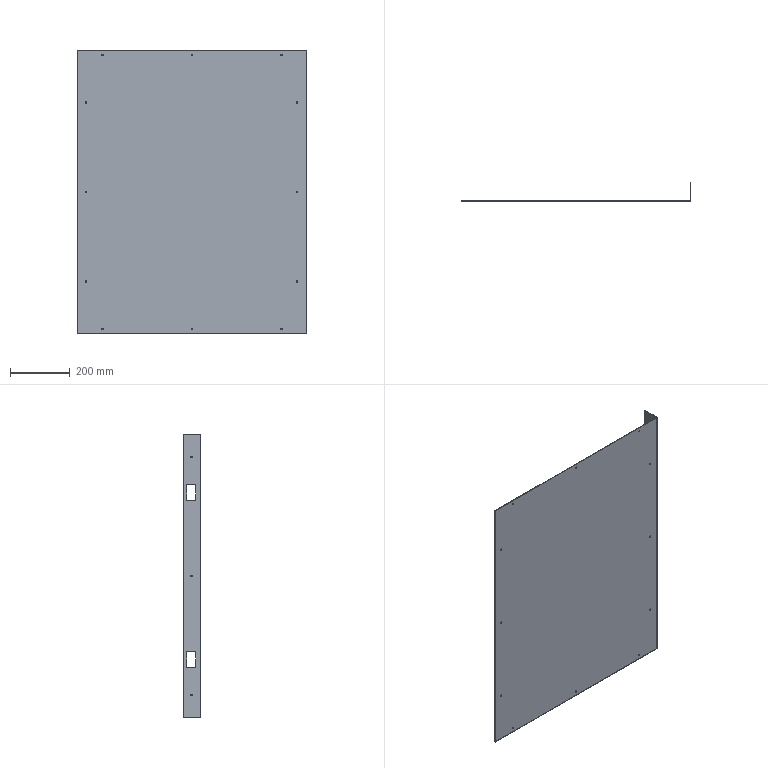Part | SolidWorks | features ICE 3, Extrusion 1 | 1 solid | 46 faces | box 770 x 60 x 950 mm | volume 1175242 mm3 | cylinder 30 | plane 16 | commonest cylinder face diameters 5 x30
STEP:
#1=CARTESIAN_POINT('',(85.,-58.5,17.5));
#2=VERTEX_POINT('',#1);
#3=CARTESIAN_POINT('',(85.,-58.5,12.5));
#4=VERTEX_POINT('',#3);
#5=CARTESIAN_POINT('',(85.,-58.5,15.));
#6=DIRECTION('',(0.,-1.,0.));
#7=DIRECTION('',(0.,0.,1.));
#8=AXIS2_PLACEMENT_3D('',#5,#6,#7);
#9=CIRCLE('',#8,2.5);
#10=EDGE_CURVE('',#2,#4,#9,.T.);
#11=ORIENTED_EDGE('',*,*,#10,.F.);
#12=CARTESIAN_POINT('',(85.,-60.,17.5));
#13=VERTEX_POINT('',#12);
#14=CARTESIAN_POINT('',(85.,-58.5,17.5));
#15=DIRECTION('',(0.,-1.,0.));
#16=VECTOR('',#15,1000.);
#17=LINE('',#14,#16);
#18=EDGE_CURVE('',#2,#13,#17,.T.);
#19=ORIENTED_EDGE('',*,*,#18,.T.);
#20=CARTESIAN_POINT('',(85.,-60.,12.5));
#21=VERTEX_POINT('',#20);
#22=CARTESIAN_POINT('',(85.,-60.,15.));
#23=DIRECTION('',(0.,-1.,0.));
#24=DIRECTION('',(0.,0.,1.));
#25=AXIS2_PLACEMENT_3D('',#22,#23,#24);
#26=CIRCLE('',#25,2.5);
#27=EDGE_CURVE('',#13,#21,#26,.T.);
#28=ORIENTED_EDGE('',*,*,#27,.T.);
#29=CARTESIAN_POINT('',(85.,-58.5,12.5));
#30=DIRECTION('',(0.,-1.,0.));
#31=VECTOR('',#30,1000.);
#32=LINE('',#29,#31);
#33=EDGE_CURVE('',#4,#21,#32,.T.);
#34=ORIENTED_EDGE('',*,*,#33,.F.);
#35=EDGE_LOOP('',(#11,#19,#28,#34));
#36=FACE_OUTER_BOUND('',#35,.T.);
#37=CARTESIAN_POINT('',(85.,-58.5,15.));
#38=DIRECTION('',(0.,-1.,0.));
#39=DIRECTION('',(0.,0.,-1.));
#40=AXIS2_PLACEMENT_3D('',#37,#38,#39);
#41=CYLINDRICAL_SURFACE('',#40,2.5);
#42=ADVANCED_FACE('',(#36),#41,.F.);
#43=CARTESIAN_POINT('',(685.,-58.5,17.5));
#44=VERTEX_POINT('',#43);
#45=CARTESIAN_POINT('',(685.,-58.5,12.5));
#46=VERTEX_POINT('',#45);
#47=CARTESIAN_POINT('',(685.,-58.5,15.));
#48=DIRECTION('',(0.,-1.,0.));
#49=DIRECTION('',(0.,0.,1.));
#50=AXIS2_PLACEMENT_3D('',#47,#48,#49);
#51=CIRCLE('',#50,2.5);
#52=EDGE_CURVE('',#44,#46,#51,.T.);
#53=ORIENTED_EDGE('',*,*,#52,.F.);
#54=CARTESIAN_POINT('',(685.,-60.,17.5));
#55=VERTEX_POINT('',#54);
#56=CARTESIAN_POINT('',(685.,-58.5,17.5));
#57=DIRECTION('',(0.,-1.,0.));
#58=VECTOR('',#57,1000.);
#59=LINE('',#56,#58);
#60=EDGE_CURVE('',#44,#55,#59,.T.);
#61=ORIENTED_EDGE('',*,*,#60,.T.);
#62=CARTESIAN_POINT('',(685.,-60.,12.5));
#63=VERTEX_POINT('',#62);
#64=CARTESIAN_POINT('',(685.,-60.,15.));
#65=DIRECTION('',(0.,-1.,0.));
#66=DIRECTION('',(0.,0.,1.));
#67=AXIS2_PLACEMENT_3D('',#64,#65,#66);
#68=CIRCLE('',#67,2.5);
#69=EDGE_CURVE('',#55,#63,#68,.T.);
#70=ORIENTED_EDGE('',*,*,#69,.T.);
#71=CARTESIAN_POINT('',(685.,-58.5,12.5));
#72=DIRECTION('',(0.,-1.,0.));
#73=VECTOR('',#72,1000.);
#74=LINE('',#71,#73);
#75=EDGE_CURVE('',#46,#63,#74,.T.);
#76=ORIENTED_EDGE('',*,*,#75,.F.);
#77=EDGE_LOOP('',(#53,#61,#70,#76));
#78=FACE_OUTER_BOUND('',#77,.T.);
#79=CARTESIAN_POINT('',(685.,-58.5,15.));
#80=DIRECTION('',(0.,-1.,0.));
#81=DIRECTION('',(0.,0.,-1.));
#82=AXIS2_PLACEMENT_3D('',#79,#80,#81);
#83=CYLINDRICAL_SURFACE('',#82,2.5);
#84=ADVANCED_FACE('',(#78),#83,.F.);
#85=CARTESIAN_POINT('',(385.,-58.5,17.5));
#86=VERTEX_POINT('',#85);
#87=CARTESIAN_POINT('',(385.,-58.5,12.5));
#88=VERTEX_POINT('',#87);
#89=CARTESIAN_POINT('',(385.,-58.5,15.));
#90=DIRECTION('',(0.,-1.,0.));
#91=DIRECTION('',(0.,0.,1.));
#92=AXIS2_PLACEMENT_3D('',#89,#90,#91);
#93=CIRCLE('',#92,2.5);
#94=EDGE_CURVE('',#86,#88,#93,.T.);
#95=ORIENTED_EDGE('',*,*,#94,.F.);
#96=CARTESIAN_POINT('',(385.,-60.,17.5));
#97=VERTEX_POINT('',#96);
#98=CARTESIAN_POINT('',(385.,-58.5,17.5));
#99=DIRECTION('',(0.,-1.,0.));
#100=VECTOR('',#99,1000.);
#101=LINE('',#98,#100);
#102=EDGE_CURVE('',#86,#97,#101,.T.);
#103=ORIENTED_EDGE('',*,*,#102,.T.);
#104=CARTESIAN_POINT('',(385.,-60.,12.5));
#105=VERTEX_POINT('',#104);
#106=CARTESIAN_POINT('',(385.,-60.,15.));
#107=DIRECTION('',(0.,-1.,0.));
#108=DIRECTION('',(0.,0.,1.));
#109=AXIS2_PLACEMENT_3D('',#106,#107,#108);
#110=CIRCLE('',#109,2.5);
#111=EDGE_CURVE('',#97,#105,#110,.T.);
#112=ORIENTED_EDGE('',*,*,#111,.T.);
#113=CARTESIAN_POINT('',(385.,-58.5,12.5));
#114=DIRECTION('',(0.,-1.,0.));
#115=VECTOR('',#114,1000.);
#116=LINE('',#113,#115);
#117=EDGE_CURVE('',#88,#105,#116,.T.);
#118=ORIENTED_EDGE('',*,*,#117,.F.);
#119=EDGE_LOOP('',(#95,#103,#112,#118));
#120=FACE_OUTER_BOUND('',#119,.T.);
#121=CARTESIAN_POINT('',(385.,-58.5,15.));
#122=DIRECTION('',(0.,-1.,0.));
#123=DIRECTION('',(0.,0.,-1.));
#124=AXIS2_PLACEMENT_3D('',#121,#122,#123);
#125=CYLINDRICAL_SURFACE('',#124,2.5);
#126=ADVANCED_FACE('',(#120),#125,.F.);
#127=CARTESIAN_POINT('',(737.,-58.5,777.5));
#128=VERTEX_POINT('',#127);
#129=CARTESIAN_POINT('',(737.,-58.5,772.5));
#130=VERTEX_POINT('',#129);
#131=CARTESIAN_POINT('',(737.,-58.5,775.));
#132=DIRECTION('',(0.,-1.,0.));
#133=DIRECTION('',(0.,0.,-1.));
#134=AXIS2_PLACEMENT_3D('',#131,#132,#133);
#135=CIRCLE('',#134,2.5);
#136=EDGE_CURVE('',#128,#130,#135,.T.);
#137=ORIENTED_EDGE('',*,*,#136,.F.);
#138=CARTESIAN_POINT('',(737.,-60.,777.5));
#139=VERTEX_POINT('',#138);
#140=CARTESIAN_POINT('',(737.,-58.5,777.5));
#141=DIRECTION('',(0.,-1.,0.));
#142=VECTOR('',#141,1000.);
#143=LINE('',#140,#142);
#144=EDGE_CURVE('',#128,#139,#143,.T.);
#145=ORIENTED_EDGE('',*,*,#144,.T.);
#146=CARTESIAN_POINT('',(737.,-60.,772.5));
#147=VERTEX_POINT('',#146);
#148=CARTESIAN_POINT('',(737.,-60.,775.));
#149=DIRECTION('',(0.,-1.,0.));
#150=DIRECTION('',(0.,0.,-1.));
#151=AXIS2_PLACEMENT_3D('',#148,#149,#150);
#152=CIRCLE('',#151,2.5);
#153=EDGE_CURVE('',#139,#147,#152,.T.);
#154=ORIENTED_EDGE('',*,*,#153,.T.);
#155=CARTESIAN_POINT('',(737.,-58.5,772.5));
#156=DIRECTION('',(0.,-1.,0.));
#157=VECTOR('',#156,1000.);
#158=LINE('',#155,#157);
#159=EDGE_CURVE('',#130,#147,#158,.T.);
#160=ORIENTED_EDGE('',*,*,#159,.F.);
#161=EDGE_LOOP('',(#137,#145,#154,#160));
#162=FACE_OUTER_BOUND('',#161,.T.);
#163=CARTESIAN_POINT('',(737.,-58.5,775.));
#164=DIRECTION('',(0.,-1.,0.));
#165=DIRECTION('',(0.,0.,-1.));
#166=AXIS2_PLACEMENT_3D('',#163,#164,#165);
#167=CYLINDRICAL_SURFACE('',#166,2.5);
#168=ADVANCED_FACE('',(#162),#167,.F.);
#169=CARTESIAN_POINT('',(737.,-58.5,177.5));
#170=VERTEX_POINT('',#169);
#171=CARTESIAN_POINT('',(737.,-58.5,172.5));
#172=VERTEX_POINT('',#171);
#173=CARTESIAN_POINT('',(737.,-58.5,175.));
#174=DIRECTION('',(0.,-1.,0.));
#175=DIRECTION('',(0.,0.,-1.));
#176=AXIS2_PLACEMENT_3D('',#173,#174,#175);
#177=CIRCLE('',#176,2.5);
#178=EDGE_CURVE('',#170,#172,#177,.T.);
#179=ORIENTED_EDGE('',*,*,#178,.F.);
#180=CARTESIAN_POINT('',(737.,-60.,177.5));
#181=VERTEX_POINT('',#180);
#182=CARTESIAN_POINT('',(737.,-58.5,177.5));
#183=DIRECTION('',(0.,-1.,0.));
#184=VECTOR('',#183,1000.);
#185=LINE('',#182,#184);
#186=EDGE_CURVE('',#170,#181,#185,.T.);
#187=ORIENTED_EDGE('',*,*,#186,.T.);
#188=CARTESIAN_POINT('',(737.,-60.,172.5));
#189=VERTEX_POINT('',#188);
#190=CARTESIAN_POINT('',(737.,-60.,175.));
#191=DIRECTION('',(0.,-1.,0.));
#192=DIRECTION('',(0.,0.,-1.));
#193=AXIS2_PLACEMENT_3D('',#190,#191,#192);
#194=CIRCLE('',#193,2.5);
#195=EDGE_CURVE('',#181,#189,#194,.T.);
#196=ORIENTED_EDGE('',*,*,#195,.T.);
#197=CARTESIAN_POINT('',(737.,-58.5,172.5));
#198=DIRECTION('',(0.,-1.,0.));
#199=VECTOR('',#198,1000.);
#200=LINE('',#197,#199);
#201=EDGE_CURVE('',#172,#189,#200,.T.);
#202=ORIENTED_EDGE('',*,*,#201,.F.);
#203=EDGE_LOOP('',(#179,#187,#196,#202));
#204=FACE_OUTER_BOUND('',#203,.T.);
#205=CARTESIAN_POINT('',(737.,-58.5,175.));
#206=DIRECTION('',(0.,-1.,0.));
#207=DIRECTION('',(0.,0.,-1.));
#208=AXIS2_PLACEMENT_3D('',#205,#206,#207);
#209=CYLINDRICAL_SURFACE('',#208,2.5);
#210=ADVANCED_FACE('',(#204),#209,.F.);
#211=CARTESIAN_POINT('',(385.,-58.5,937.5));
#212=VERTEX_POINT('',#211);
#213=CARTESIAN_POINT('',(385.,-58.5,932.5));
#214=VERTEX_POINT('',#213);
#215=CARTESIAN_POINT('',(385.,-58.5,935.));
#216=DIRECTION('',(0.,-1.,0.));
#217=DIRECTION('',(0.,0.,-1.));
#218=AXIS2_PLACEMENT_3D('',#215,#216,#217);
#219=CIRCLE('',#218,2.5);
#220=EDGE_CURVE('',#212,#214,#219,.T.);
#221=ORIENTED_EDGE('',*,*,#220,.F.);
#222=CARTESIAN_POINT('',(385.,-60.,937.5));
#223=VERTEX_POINT('',#222);
#224=CARTESIAN_POINT('',(385.,-58.5,937.5));
#225=DIRECTION('',(0.,-1.,0.));
#226=VECTOR('',#225,1000.);
#227=LINE('',#224,#226);
#228=EDGE_CURVE('',#212,#223,#227,.T.);
#229=ORIENTED_EDGE('',*,*,#228,.T.);
#230=CARTESIAN_POINT('',(385.,-60.,932.5));
#231=VERTEX_POINT('',#230);
#232=CARTESIAN_POINT('',(385.,-60.,935.));
#233=DIRECTION('',(0.,-1.,0.));
#234=DIRECTION('',(0.,0.,-1.));
#235=AXIS2_PLACEMENT_3D('',#232,#233,#234);
#236=CIRCLE('',#235,2.5);
#237=EDGE_CURVE('',#223,#231,#236,.T.);
#238=ORIENTED_EDGE('',*,*,#237,.T.);
#239=CARTESIAN_POINT('',(385.,-58.5,932.5));
#240=DIRECTION('',(0.,-1.,0.));
#241=VECTOR('',#240,1000.);
#242=LINE('',#239,#241);
#243=EDGE_CURVE('',#214,#231,#242,.T.);
#244=ORIENTED_EDGE('',*,*,#243,.F.);
#245=EDGE_LOOP('',(#221,#229,#238,#244));
#246=FACE_OUTER_BOUND('',#245,.T.);
#247=CARTESIAN_POINT('',(385.,-58.5,935.));
#248=DIRECTION('',(0.,-1.,0.));
#249=DIRECTION('',(0.,0.,-1.));
#250=AXIS2_PLACEMENT_3D('',#247,#248,#249);
#251=CYLINDRICAL_SURFACE('',#250,2.5);
#252=ADVANCED_FACE('',(#246),#251,.F.);
#253=CARTESIAN_POINT('',(30.,-58.5,477.5));
#254=VERTEX_POINT('',#253);
#255=CARTESIAN_POINT('',(30.,-58.5,472.5));
#256=VERTEX_POINT('',#255);
#257=CARTESIAN_POINT('',(30.,-58.5,475.));
#258=DIRECTION('',(0.,-1.,0.));
#259=DIRECTION('',(0.,0.,-1.));
#260=AXIS2_PLACEMENT_3D('',#257,#258,#259);
#261=CIRCLE('',#260,2.5);
#262=EDGE_CURVE('',#254,#256,#261,.T.);
#263=ORIENTED_EDGE('',*,*,#262,.F.);
#264=CARTESIAN_POINT('',(30.,-60.,477.5));
#265=VERTEX_POINT('',#264);
#266=CARTESIAN_POINT('',(30.,-58.5,477.5));
#267=DIRECTION('',(0.,-1.,0.));
#268=VECTOR('',#267,1000.);
#269=LINE('',#266,#268);
#270=EDGE_CURVE('',#254,#265,#269,.T.);
#271=ORIENTED_EDGE('',*,*,#270,.T.);
#272=CARTESIAN_POINT('',(30.,-60.,472.5));
#273=VERTEX_POINT('',#272);
#274=CARTESIAN_POINT('',(30.,-60.,475.));
#275=DIRECTION('',(0.,-1.,0.));
#276=DIRECTION('',(0.,0.,-1.));
#277=AXIS2_PLACEMENT_3D('',#274,#275,#276);
#278=CIRCLE('',#277,2.5);
#279=EDGE_CURVE('',#265,#273,#278,.T.);
#280=ORIENTED_EDGE('',*,*,#279,.T.);
#281=CARTESIAN_POINT('',(30.,-58.5,472.5));
#282=DIRECTION('',(0.,-1.,0.));
#283=VECTOR('',#282,1000.);
#284=LINE('',#281,#283);
#285=EDGE_CURVE('',#256,#273,#284,.T.);
#286=ORIENTED_EDGE('',*,*,#285,.F.);
#287=EDGE_LOOP('',(#263,#271,#280,#286));
#288=FACE_OUTER_BOUND('',#287,.T.);
#289=CARTESIAN_POINT('',(30.,-58.5,475.));
#290=DIRECTION('',(0.,-1.,0.));
#291=DIRECTION('',(0.,0.,-1.));
#292=AXIS2_PLACEMENT_3D('',#289,#290,#291);
#293=CYLINDRICAL_SURFACE('',#292,2.5);
#294=ADVANCED_FACE('',(#288),#293,.F.);
#295=CARTESIAN_POINT('',(30.,-58.5,777.5));
#296=VERTEX_POINT('',#295);
#297=CARTESIAN_POINT('',(30.,-58.5,772.5));
#298=VERTEX_POINT('',#297);
#299=CARTESIAN_POINT('',(30.,-58.5,775.));
#300=DIRECTION('',(0.,-1.,0.));
#301=DIRECTION('',(0.,0.,-1.));
#302=AXIS2_PLACEMENT_3D('',#299,#300,#301);
#303=CIRCLE('',#302,2.5);
#304=EDGE_CURVE('',#296,#298,#303,.T.);
#305=ORIENTED_EDGE('',*,*,#304,.F.);
#306=CARTESIAN_POINT('',(30.,-60.,777.5));
#307=VERTEX_POINT('',#306);
#308=CARTESIAN_POINT('',(30.,-58.5,777.5));
#309=DIRECTION('',(0.,-1.,0.));
#310=VECTOR('',#309,1000.);
#311=LINE('',#308,#310);
#312=EDGE_CURVE('',#296,#307,#311,.T.);
#313=ORIENTED_EDGE('',*,*,#312,.T.);
#314=CARTESIAN_POINT('',(30.,-60.,772.5));
#315=VERTEX_POINT('',#314);
#316=CARTESIAN_POINT('',(30.,-60.,775.));
#317=DIRECTION('',(0.,-1.,0.));
#318=DIRECTION('',(0.,0.,-1.));
#319=AXIS2_PLACEMENT_3D('',#316,#317,#318);
#320=CIRCLE('',#319,2.5);
#321=EDGE_CURVE('',#307,#315,#320,.T.);
#322=ORIENTED_EDGE('',*,*,#321,.T.);
#323=CARTESIAN_POINT('',(30.,-58.5,772.5));
#324=DIRECTION('',(0.,-1.,0.));
#325=VECTOR('',#324,1000.);
#326=LINE('',#323,#325);
#327=EDGE_CURVE('',#298,#315,#326,.T.);
#328=ORIENTED_EDGE('',*,*,#327,.F.);
#329=EDGE_LOOP('',(#305,#313,#322,#328));
#330=FACE_OUTER_BOUND('',#329,.T.);
#331=CARTESIAN_POINT('',(30.,-58.5,775.));
#332=DIRECTION('',(0.,-1.,0.));
#333=DIRECTION('',(0.,0.,-1.));
#334=AXIS2_PLACEMENT_3D('',#331,#332,#333);
#335=CYLINDRICAL_SURFACE('',#334,2.5);
#336=ADVANCED_FACE('',(#330),#335,.F.);
#337=CARTESIAN_POINT('',(30.,-58.5,177.5));
#338=VERTEX_POINT('',#337);
#339=CARTESIAN_POINT('',(30.,-58.5,172.5));
#340=VERTEX_POINT('',#339);
#341=CARTESIAN_POINT('',(30.,-58.5,175.));
#342=DIRECTION('',(0.,-1.,0.));
#343=DIRECTION('',(0.,0.,-1.));
#344=AXIS2_PLACEMENT_3D('',#341,#342,#343);
#345=CIRCLE('',#344,2.5);
#346=EDGE_CURVE('',#338,#340,#345,.T.);
#347=ORIENTED_EDGE('',*,*,#346,.F.);
#348=CARTESIAN_POINT('',(30.,-60.,177.5));
#349=VERTEX_POINT('',#348);
#350=CARTESIAN_POINT('',(30.,-58.5,177.5));
#351=DIRECTION('',(0.,-1.,0.));
#352=VECTOR('',#351,1000.);
#353=LINE('',#350,#352);
#354=EDGE_CURVE('',#338,#349,#353,.T.);
#355=ORIENTED_EDGE('',*,*,#354,.T.);
#356=CARTESIAN_POINT('',(30.,-60.,172.5));
#357=VERTEX_POINT('',#356);
#358=CARTESIAN_POINT('',(30.,-60.,175.));
#359=DIRECTION('',(0.,-1.,0.));
#360=DIRECTION('',(0.,0.,-1.));
#361=AXIS2_PLACEMENT_3D('',#358,#359,#360);
#362=CIRCLE('',#361,2.5);
#363=EDGE_CURVE('',#349,#357,#362,.T.);
#364=ORIENTED_EDGE('',*,*,#363,.T.);
#365=CARTESIAN_POINT('',(30.,-58.5,172.5));
#366=DIRECTION('',(0.,-1.,0.));
#367=VECTOR('',#366,1000.);
#368=LINE('',#365,#367);
#369=EDGE_CURVE('',#340,#357,#368,.T.);
#370=ORIENTED_EDGE('',*,*,#369,.F.);
#371=EDGE_LOOP('',(#347,#355,#364,#370));
#372=FACE_OUTER_BOUND('',#371,.T.);
#373=CARTESIAN_POINT('',(30.,-58.5,175.));
#374=DIRECTION('',(0.,-1.,0.));
#375=DIRECTION('',(0.,0.,-1.));
#376=AXIS2_PLACEMENT_3D('',#373,#374,#375);
#377=CYLINDRICAL_SURFACE('',#376,2.5);
#378=ADVANCED_FACE('',(#372),#377,.F.);
#379=CARTESIAN_POINT('',(685.,-58.5,937.5));
#380=VERTEX_POINT('',#379);
#381=CARTESIAN_POINT('',(685.,-58.5,932.5));
#382=VERTEX_POINT('',#381);
#383=CARTESIAN_POINT('',(685.,-58.5,935.));
#384=DIRECTION('',(0.,-1.,0.));
#385=DIRECTION('',(0.,0.,-1.));
#386=AXIS2_PLACEMENT_3D('',#383,#384,#385);
#387=CIRCLE('',#386,2.5);
#388=EDGE_CURVE('',#380,#382,#387,.T.);
#389=ORIENTED_EDGE('',*,*,#388,.F.);
#390=CARTESIAN_POINT('',(685.,-60.,937.5));
#391=VERTEX_POINT('',#390);
#392=CARTESIAN_POINT('',(685.,-58.5,937.5));
#393=DIRECTION('',(0.,-1.,0.));
#394=VECTOR('',#393,1000.);
#395=LINE('',#392,#394);
#396=EDGE_CURVE('',#380,#391,#395,.T.);
#397=ORIENTED_EDGE('',*,*,#396,.T.);
#398=CARTESIAN_POINT('',(685.,-60.,932.5));
#399=VERTEX_POINT('',#398);
#400=CARTESIAN_POINT('',(685.,-60.,935.));
#401=DIRECTION('',(0.,-1.,0.));
#402=DIRECTION('',(0.,0.,-1.));
#403=AXIS2_PLACEMENT_3D('',#400,#401,#402);
#404=CIRCLE('',#403,2.5);
#405=EDGE_CURVE('',#391,#399,#404,.T.);
#406=ORIENTED_EDGE('',*,*,#405,.T.);
#407=CARTESIAN_POINT('',(685.,-58.5,932.5));
#408=DIRECTION('',(0.,-1.,0.));
#409=VECTOR('',#408,1000.);
#410=LINE('',#407,#409);
#411=EDGE_CURVE('',#382,#399,#410,.T.);
#412=ORIENTED_EDGE('',*,*,#411,.F.);
#413=EDGE_LOOP('',(#389,#397,#406,#412));
#414=FACE_OUTER_BOUND('',#413,.T.);
#415=CARTESIAN_POINT('',(685.,-58.5,935.));
#416=DIRECTION('',(0.,-1.,0.));
#417=DIRECTION('',(0.,0.,-1.));
#418=AXIS2_PLACEMENT_3D('',#415,#416,#417);
#419=CYLINDRICAL_SURFACE('',#418,2.5);
#420=ADVANCED_FACE('',(#414),#419,.F.);
#421=CARTESIAN_POINT('',(85.,-58.5,937.5));
#422=VERTEX_POINT('',#421);
#423=CARTESIAN_POINT('',(85.,-58.5,932.5));
#424=VERTEX_POINT('',#423);
#425=CARTESIAN_POINT('',(85.,-58.5,935.));
#426=DIRECTION('',(0.,-1.,0.));
#427=DIRECTION('',(0.,0.,-1.));
#428=AXIS2_PLACEMENT_3D('',#425,#426,#427);
#429=CIRCLE('',#428,2.5);
#430=EDGE_CURVE('',#422,#424,#429,.T.);
#431=ORIENTED_EDGE('',*,*,#430,.F.);
#432=CARTESIAN_POINT('',(85.,-60.,937.5));
#433=VERTEX_POINT('',#432);
#434=CARTESIAN_POINT('',(85.,-58.5,937.5));
#435=DIRECTION('',(0.,-1.,0.));
#436=VECTOR('',#435,1000.);
#437=LINE('',#434,#436);
#438=EDGE_CURVE('',#422,#433,#437,.T.);
#439=ORIENTED_EDGE('',*,*,#438,.T.);
#440=CARTESIAN_POINT('',(85.,-60.,932.5));
#441=VERTEX_POINT('',#440);
#442=CARTESIAN_POINT('',(85.,-60.,935.));
#443=DIRECTION('',(0.,-1.,0.));
#444=DIRECTION('',(0.,0.,-1.));
#445=AXIS2_PLACEMENT_3D('',#442,#443,#444);
#446=CIRCLE('',#445,2.5);
#447=EDGE_CURVE('',#433,#441,#446,.T.);
#448=ORIENTED_EDGE('',*,*,#447,.T.);
#449=CARTESIAN_POINT('',(85.,-58.5,932.5));
#450=DIRECTION('',(0.,-1.,0.));
#451=VECTOR('',#450,1000.);
#452=LINE('',#449,#451);
#453=EDGE_CURVE('',#424,#441,#452,.T.);
#454=ORIENTED_EDGE('',*,*,#453,.F.);
#455=EDGE_LOOP('',(#431,#439,#448,#454));
#456=FACE_OUTER_BOUND('',#455,.T.);
#457=CARTESIAN_POINT('',(85.,-58.5,935.));
#458=DIRECTION('',(0.,-1.,0.));
#459=DIRECTION('',(0.,0.,-1.));
#460=AXIS2_PLACEMENT_3D('',#457,#458,#459);
#461=CYLINDRICAL_SURFACE('',#460,2.5);
#462=ADVANCED_FACE('',(#456),#461,.F.);
#463=CARTESIAN_POINT('',(737.,-58.5,477.5));
#464=VERTEX_POINT('',#463);
#465=CARTESIAN_POINT('',(737.,-58.5,472.5));
#466=VERTEX_POINT('',#465);
#467=CARTESIAN_POINT('',(737.,-58.5,475.));
#468=DIRECTION('',(0.,-1.,0.));
#469=DIRECTION('',(0.,0.,-1.));
#470=AXIS2_PLACEMENT_3D('',#467,#468,#469);
#471=CIRCLE('',#470,2.5);
#472=EDGE_CURVE('',#464,#466,#471,.T.);
#473=ORIENTED_EDGE('',*,*,#472,.F.);
#474=CARTESIAN_POINT('',(737.,-60.,477.5));
#475=VERTEX_POINT('',#474);
#476=CARTESIAN_POINT('',(737.,-58.5,477.5));
#477=DIRECTION('',(0.,-1.,0.));
#478=VECTOR('',#477,1000.);
#479=LINE('',#476,#478);
#480=EDGE_CURVE('',#464,#475,#479,.T.);
#481=ORIENTED_EDGE('',*,*,#480,.T.);
#482=CARTESIAN_POINT('',(737.,-60.,472.5));
#483=VERTEX_POINT('',#482);
#484=CARTESIAN_POINT('',(737.,-60.,475.));
#485=DIRECTION('',(0.,-1.,0.));
#486=DIRECTION('',(0.,0.,-1.));
#487=AXIS2_PLACEMENT_3D('',#484,#485,#486);
#488=CIRCLE('',#487,2.5);
#489=EDGE_CURVE('',#475,#483,#488,.T.);
#490=ORIENTED_EDGE('',*,*,#489,.T.);
#491=CARTESIAN_POINT('',(737.,-58.5,472.5));
#492=DIRECTION('',(0.,-1.,0.));
#493=VECTOR('',#492,1000.);
#494=LINE('',#491,#493);
#495=EDGE_CURVE('',#466,#483,#494,.T.);
#496=ORIENTED_EDGE('',*,*,#495,.F.);
#497=EDGE_LOOP('',(#473,#481,#490,#496));
#498=FACE_OUTER_BOUND('',#497,.T.);
#499=CARTESIAN_POINT('',(737.,-58.5,475.));
#500=DIRECTION('',(0.,-1.,0.));
#501=DIRECTION('',(0.,0.,-1.));
#502=AXIS2_PLACEMENT_3D('',#499,#500,#501);
#503=CYLINDRICAL_SURFACE('',#502,2.5);
#504=ADVANCED_FACE('',(#498),#503,.F.);
#505=CARTESIAN_POINT('',(768.5,-28.5,877.5));
#506=VERTEX_POINT('',#505);
#507=CARTESIAN_POINT('',(768.5,-28.5,872.5));
#508=VERTEX_POINT('',#507);
#509=CARTESIAN_POINT('',(768.5,-28.5,875.));
#510=DIRECTION('',(1.,0.,0.));
#511=DIRECTION('',(0.,0.,-1.));
#512=AXIS2_PLACEMENT_3D('',#509,#510,#511);
#513=CIRCLE('',#512,2.5);
#514=EDGE_CURVE('',#506,#508,#513,.T.);
#515=ORIENTED_EDGE('',*,*,#514,.F.);
#516=CARTESIAN_POINT('',(770.,-28.5,877.5));
#517=VERTEX_POINT('',#516);
#518=CARTESIAN_POINT('',(-586.5,-28.5,877.5));
#519=DIRECTION('',(1.,0.,0.));
#520=VECTOR('',#519,1000.);
#521=LINE('',#518,#520);
#522=EDGE_CURVE('',#506,#517,#521,.T.);
#523=ORIENTED_EDGE('',*,*,#522,.T.);
#524=CARTESIAN_POINT('',(770.,-28.5,872.5));
#525=VERTEX_POINT('',#524);
#526=CARTESIAN_POINT('',(770.,-28.5,875.));
#527=DIRECTION('',(1.,0.,0.));
#528=DIRECTION('',(0.,0.,-1.));
#529=AXIS2_PLACEMENT_3D('',#526,#527,#528);
#530=CIRCLE('',#529,2.5);
#531=EDGE_CURVE('',#517,#525,#530,.T.);
#532=ORIENTED_EDGE('',*,*,#531,.T.);
#533=CARTESIAN_POINT('',(-586.5,-28.5,872.5));
#534=DIRECTION('',(1.,0.,0.));
#535=VECTOR('',#534,1000.);
#536=LINE('',#533,#535);
#537=EDGE_CURVE('',#508,#525,#536,.T.);
#538=ORIENTED_EDGE('',*,*,#537,.F.);
#539=EDGE_LOOP('',(#515,#523,#532,#538));
#540=FACE_OUTER_BOUND('',#539,.T.);
#541=CARTESIAN_POINT('',(-586.5,-28.5,875.));
#542=DIRECTION('',(1.,0.,0.));
#543=DIRECTION('',(0.,0.,-1.));
#544=AXIS2_PLACEMENT_3D('',#541,#542,#543);
#545=CYLINDRICAL_SURFACE('',#544,2.5);
#546=ADVANCED_FACE('',(#540),#545,.F.);
#547=CARTESIAN_POINT('',(768.5,-28.5,477.5));
#548=VERTEX_POINT('',#547);
#549=CARTESIAN_POINT('',(768.5,-28.5,472.5));
#550=VERTEX_POINT('',#549);
#551=CARTESIAN_POINT('',(768.5,-28.5,475.));
#552=DIRECTION('',(1.,0.,0.));
#553=DIRECTION('',(0.,0.,-1.));
#554=AXIS2_PLACEMENT_3D('',#551,#552,#553);
#555=CIRCLE('',#554,2.5);
#556=EDGE_CURVE('',#548,#550,#555,.T.);
#557=ORIENTED_EDGE('',*,*,#556,.F.);
#558=CARTESIAN_POINT('',(770.,-28.5,477.5));
#559=VERTEX_POINT('',#558);
#560=CARTESIAN_POINT('',(-586.5,-28.5,477.5));
#561=DIRECTION('',(1.,0.,0.));
#562=VECTOR('',#561,1000.);
#563=LINE('',#560,#562);
#564=EDGE_CURVE('',#548,#559,#563,.T.);
#565=ORIENTED_EDGE('',*,*,#564,.T.);
#566=CARTESIAN_POINT('',(770.,-28.5,472.5));
#567=VERTEX_POINT('',#566);
#568=CARTESIAN_POINT('',(770.,-28.5,475.));
#569=DIRECTION('',(1.,0.,0.));
#570=DIRECTION('',(0.,0.,-1.));
#571=AXIS2_PLACEMENT_3D('',#568,#569,#570);
#572=CIRCLE('',#571,2.5);
#573=EDGE_CURVE('',#559,#567,#572,.T.);
#574=ORIENTED_EDGE('',*,*,#573,.T.);
#575=CARTESIAN_POINT('',(-586.5,-28.5,472.5));
#576=DIRECTION('',(1.,0.,0.));
#577=VECTOR('',#576,1000.);
#578=LINE('',#575,#577);
#579=EDGE_CURVE('',#550,#567,#578,.T.);
#580=ORIENTED_EDGE('',*,*,#579,.F.);
#581=EDGE_LOOP('',(#557,#565,#574,#580));
#582=FACE_OUTER_BOUND('',#581,.T.);
#583=CARTESIAN_POINT('',(-586.5,-28.5,475.));
#584=DIRECTION('',(1.,0.,0.));
#585=DIRECTION('',(0.,0.,-1.));
#586=AXIS2_PLACEMENT_3D('',#583,#584,#585);
#587=CYLINDRICAL_SURFACE('',#586,2.5);
#588=ADVANCED_FACE('',(#582),#587,.F.);
#589=CARTESIAN_POINT('',(768.5,-28.5,77.5));
#590=VERTEX_POINT('',#589);
#591=CARTESIAN_POINT('',(768.5,-28.5,72.5));
#592=VERTEX_POINT('',#591);
#593=CARTESIAN_POINT('',(768.5,-28.5,75.));
#594=DIRECTION('',(1.,0.,0.));
#595=DIRECTION('',(0.,0.,-1.));
#596=AXIS2_PLACEMENT_3D('',#593,#594,#595);
#597=CIRCLE('',#596,2.5);
#598=EDGE_CURVE('',#590,#592,#597,.T.);
#599=ORIENTED_EDGE('',*,*,#598,.F.);
#600=CARTESIAN_POINT('',(770.,-28.5,77.5));
#601=VERTEX_POINT('',#600);
#602=CARTESIAN_POINT('',(-586.5,-28.5,77.5));
#603=DIRECTION('',(1.,0.,0.));
#604=VECTOR('',#603,1000.);
#605=LINE('',#602,#604);
#606=EDGE_CURVE('',#590,#601,#605,.T.);
#607=ORIENTED_EDGE('',*,*,#606,.T.);
#608=CARTESIAN_POINT('',(770.,-28.5,72.5));
#609=VERTEX_POINT('',#608);
#610=CARTESIAN_POINT('',(770.,-28.5,75.));
#611=DIRECTION('',(1.,0.,0.));
#612=DIRECTION('',(0.,0.,-1.));
#613=AXIS2_PLACEMENT_3D('',#610,#611,#612);
#614=CIRCLE('',#613,2.5);
#615=EDGE_CURVE('',#601,#609,#614,.T.);
#616=ORIENTED_EDGE('',*,*,#615,.T.);
#617=CARTESIAN_POINT('',(-586.5,-28.5,72.5));
#618=DIRECTION('',(1.,0.,0.));
#619=VECTOR('',#618,1000.);
#620=LINE('',#617,#619);
#621=EDGE_CURVE('',#592,#609,#620,.T.);
#622=ORIENTED_EDGE('',*,*,#621,.F.);
#623=EDGE_LOOP('',(#599,#607,#616,#622));
#624=FACE_OUTER_BOUND('',#623,.T.);
#625=CARTESIAN_POINT('',(-586.5,-28.5,75.));
#626=DIRECTION('',(1.,0.,0.));
#627=DIRECTION('',(0.,0.,-1.));
#628=AXIS2_PLACEMENT_3D('',#625,#626,#627);
#629=CYLINDRICAL_SURFACE('',#628,2.5);
#630=ADVANCED_FACE('',(#624),#629,.F.);
#631=CARTESIAN_POINT('',(0.,-58.5,950.));
#632=VERTEX_POINT('',#631);
#633=CARTESIAN_POINT('',(0.,-60.,950.));
#634=VERTEX_POINT('',#633);
#635=CARTESIAN_POINT('',(0.,0.,950.));
#636=DIRECTION('',(0.,-1.,0.));
#637=VECTOR('',#636,1000.);
#638=LINE('',#635,#637);
#639=EDGE_CURVE('',#632,#634,#638,.T.);
#640=ORIENTED_EDGE('',*,*,#639,.F.);
#641=CARTESIAN_POINT('',(0.,-58.5,0.));
#642=VERTEX_POINT('',#641);
#643=CARTESIAN_POINT('',(0.,-58.5,0.));
#644=DIRECTION('',(0.,0.,1.));
#645=VECTOR('',#644,1000.);
#646=LINE('',#643,#645);
#647=EDGE_CURVE('',#642,#632,#646,.T.);
#648=ORIENTED_EDGE('',*,*,#647,.F.);
#649=CARTESIAN_POINT('',(0.,-60.,0.));
#650=VERTEX_POINT('',#649);
#651=CARTESIAN_POINT('',(0.,0.,0.));
#652=DIRECTION('',(0.,-1.,0.));
#653=VECTOR('',#652,1000.);
#654=LINE('',#651,#653);
#655=EDGE_CURVE('',#642,#650,#654,.T.);
#656=ORIENTED_EDGE('',*,*,#655,.T.);
#657=CARTESIAN_POINT('',(0.,-60.,950.));
#658=DIRECTION('',(0.,0.,-1.));
#659=VECTOR('',#658,1000.);
#660=LINE('',#657,#659);
#661=EDGE_CURVE('',#634,#650,#660,.T.);
#662=ORIENTED_EDGE('',*,*,#661,.F.);
#663=EDGE_LOOP('',(#640,#648,#656,#662));
#664=FACE_OUTER_BOUND('',#663,.T.);
#665=CARTESIAN_POINT('',(0.,0.,950.));
#666=DIRECTION('',(1.,0.,0.));
#667=DIRECTION('',(0.,1.,0.));
#668=AXIS2_PLACEMENT_3D('',#665,#666,#667);
#669=PLANE('',#668);
#670=ADVANCED_FACE('',(#664),#669,.F.);
#671=CARTESIAN_POINT('',(85.,-60.,15.));
#672=DIRECTION('',(0.,-1.,0.));
#673=DIRECTION('',(0.,0.,1.));
#674=AXIS2_PLACEMENT_3D('',#671,#672,#673);
#675=CIRCLE('',#674,2.5);
#676=EDGE_CURVE('',#21,#13,#675,.T.);
#677=ORIENTED_EDGE('',*,*,#676,.F.);
#678=ORIENTED_EDGE('',*,*,#27,.F.);
#679=EDGE_LOOP('',(#677,#678));
#680=FACE_BOUND('',#679,.T.);
#681=CARTESIAN_POINT('',(685.,-60.,15.));
#682=DIRECTION('',(0.,-1.,0.));
#683=DIRECTION('',(0.,0.,1.));
#684=AXIS2_PLACEMENT_3D('',#681,#682,#683);
#685=CIRCLE('',#684,2.5);
#686=EDGE_CURVE('',#63,#55,#685,.T.);
#687=ORIENTED_EDGE('',*,*,#686,.F.);
#688=ORIENTED_EDGE('',*,*,#69,.F.);
#689=EDGE_LOOP('',(#687,#688));
#690=FACE_BOUND('',#689,.T.);
#691=CARTESIAN_POINT('',(385.,-60.,15.));
#692=DIRECTION('',(0.,-1.,0.));
#693=DIRECTION('',(0.,0.,1.));
#694=AXIS2_PLACEMENT_3D('',#691,#692,#693);
#695=CIRCLE('',#694,2.5);
#696=EDGE_CURVE('',#105,#97,#695,.T.);
#697=ORIENTED_EDGE('',*,*,#696,.F.);
#698=ORIENTED_EDGE('',*,*,#111,.F.);
#699=EDGE_LOOP('',(#697,#698));
#700=FACE_BOUND('',#699,.T.);
#701=CARTESIAN_POINT('',(737.,-60.,775.));
#702=DIRECTION('',(0.,-1.,0.));
#703=DIRECTION('',(0.,0.,-1.));
#704=AXIS2_PLACEMENT_3D('',#701,#702,#703);
#705=CIRCLE('',#704,2.5);
#706=EDGE_CURVE('',#147,#139,#705,.T.);
#707=ORIENTED_EDGE('',*,*,#706,.F.);
#708=ORIENTED_EDGE('',*,*,#153,.F.);
#709=EDGE_LOOP('',(#707,#708));
#710=FACE_BOUND('',#709,.T.);
#711=CARTESIAN_POINT('',(737.,-60.,175.));
#712=DIRECTION('',(0.,-1.,0.));
#713=DIRECTION('',(0.,0.,-1.));
#714=AXIS2_PLACEMENT_3D('',#711,#712,#713);
#715=CIRCLE('',#714,2.5);
#716=EDGE_CURVE('',#189,#181,#715,.T.);
#717=ORIENTED_EDGE('',*,*,#716,.F.);
#718=ORIENTED_EDGE('',*,*,#195,.F.);
#719=EDGE_LOOP('',(#717,#718));
#720=FACE_BOUND('',#719,.T.);
#721=CARTESIAN_POINT('',(385.,-60.,935.));
#722=DIRECTION('',(0.,-1.,0.));
#723=DIRECTION('',(0.,0.,-1.));
#724=AXIS2_PLACEMENT_3D('',#721,#722,#723);
#725=CIRCLE('',#724,2.5);
#726=EDGE_CURVE('',#231,#223,#725,.T.);
#727=ORIENTED_EDGE('',*,*,#726,.F.);
#728=ORIENTED_EDGE('',*,*,#237,.F.);
#729=EDGE_LOOP('',(#727,#728));
#730=FACE_BOUND('',#729,.T.);
#731=CARTESIAN_POINT('',(30.,-60.,475.));
#732=DIRECTION('',(0.,-1.,0.));
#733=DIRECTION('',(0.,0.,-1.));
#734=AXIS2_PLACEMENT_3D('',#731,#732,#733);
#735=CIRCLE('',#734,2.5);
#736=EDGE_CURVE('',#273,#265,#735,.T.);
#737=ORIENTED_EDGE('',*,*,#736,.F.);
#738=ORIENTED_EDGE('',*,*,#279,.F.);
#739=EDGE_LOOP('',(#737,#738));
#740=FACE_BOUND('',#739,.T.);
#741=CARTESIAN_POINT('',(30.,-60.,775.));
#742=DIRECTION('',(0.,-1.,0.));
#743=DIRECTION('',(0.,0.,-1.));
#744=AXIS2_PLACEMENT_3D('',#741,#742,#743);
#745=CIRCLE('',#744,2.5);
#746=EDGE_CURVE('',#315,#307,#745,.T.);
#747=ORIENTED_EDGE('',*,*,#746,.F.);
#748=ORIENTED_EDGE('',*,*,#321,.F.);
#749=EDGE_LOOP('',(#747,#748));
#750=FACE_BOUND('',#749,.T.);
#751=CARTESIAN_POINT('',(30.,-60.,175.));
#752=DIRECTION('',(0.,-1.,0.));
#753=DIRECTION('',(0.,0.,-1.));
#754=AXIS2_PLACEMENT_3D('',#751,#752,#753);
#755=CIRCLE('',#754,2.5);
#756=EDGE_CURVE('',#357,#349,#755,.T.);
#757=ORIENTED_EDGE('',*,*,#756,.F.);
#758=ORIENTED_EDGE('',*,*,#363,.F.);
#759=EDGE_LOOP('',(#757,#758));
#760=FACE_BOUND('',#759,.T.);
#761=CARTESIAN_POINT('',(685.,-60.,935.));
#762=DIRECTION('',(0.,-1.,0.));
#763=DIRECTION('',(0.,0.,-1.));
#764=AXIS2_PLACEMENT_3D('',#761,#762,#763);
#765=CIRCLE('',#764,2.5);
#766=EDGE_CURVE('',#399,#391,#765,.T.);
#767=ORIENTED_EDGE('',*,*,#766,.F.);
#768=ORIENTED_EDGE('',*,*,#405,.F.);
#769=EDGE_LOOP('',(#767,#768));
#770=FACE_BOUND('',#769,.T.);
#771=CARTESIAN_POINT('',(85.,-60.,935.));
#772=DIRECTION('',(0.,-1.,0.));
#773=DIRECTION('',(0.,0.,-1.));
#774=AXIS2_PLACEMENT_3D('',#771,#772,#773);
#775=CIRCLE('',#774,2.5);
#776=EDGE_CURVE('',#441,#433,#775,.T.);
#777=ORIENTED_EDGE('',*,*,#776,.F.);
#778=ORIENTED_EDGE('',*,*,#447,.F.);
#779=EDGE_LOOP('',(#777,#778));
#780=FACE_BOUND('',#779,.T.);
#781=CARTESIAN_POINT('',(737.,-60.,475.));
#782=DIRECTION('',(0.,-1.,0.));
#783=DIRECTION('',(0.,0.,-1.));
#784=AXIS2_PLACEMENT_3D('',#781,#782,#783);
#785=CIRCLE('',#784,2.5);
#786=EDGE_CURVE('',#483,#475,#785,.T.);
#787=ORIENTED_EDGE('',*,*,#786,.F.);
#788=ORIENTED_EDGE('',*,*,#489,.F.);
#789=EDGE_LOOP('',(#787,#788));
#790=FACE_BOUND('',#789,.T.);
#791=CARTESIAN_POINT('',(770.,-60.,0.));
#792=VERTEX_POINT('',#791);
#793=CARTESIAN_POINT('',(0.,-60.,0.));
#794=DIRECTION('',(1.,0.,0.));
#795=VECTOR('',#794,1000.);
#796=LINE('',#793,#795);
#797=EDGE_CURVE('',#650,#792,#796,.T.);
#798=ORIENTED_EDGE('',*,*,#797,.T.);
#799=CARTESIAN_POINT('',(770.,-60.,950.));
#800=VERTEX_POINT('',#799);
#801=CARTESIAN_POINT('',(770.,-60.,950.));
#802=DIRECTION('',(0.,0.,-1.));
#803=VECTOR('',#802,1000.);
#804=LINE('',#801,#803);
#805=EDGE_CURVE('',#800,#792,#804,.T.);
#806=ORIENTED_EDGE('',*,*,#805,.F.);
#807=CARTESIAN_POINT('',(0.,-60.,950.));
#808=DIRECTION('',(1.,0.,0.));
#809=VECTOR('',#808,1000.);
#810=LINE('',#807,#809);
#811=EDGE_CURVE('',#634,#800,#810,.T.);
#812=ORIENTED_EDGE('',*,*,#811,.F.);
#813=ORIENTED_EDGE('',*,*,#661,.T.);
#814=EDGE_LOOP('',(#798,#806,#812,#813));
#815=FACE_OUTER_BOUND('',#814,.T.);
#816=CARTESIAN_POINT('',(0.,-60.,950.));
#817=DIRECTION('',(0.,1.,0.));
#818=DIRECTION('',(0.,0.,1.));
#819=AXIS2_PLACEMENT_3D('',#816,#817,#818);
#820=PLANE('',#819);
#821=ADVANCED_FACE('',(#680,#690,#700,#710,#720,#730,#740,#750,#760,#770,#780,#790,#815),#820,.F.);
#822=CARTESIAN_POINT('',(770.,-28.5,875.));
#823=DIRECTION('',(1.,0.,0.));
#824=DIRECTION('',(0.,0.,-1.));
#825=AXIS2_PLACEMENT_3D('',#822,#823,#824);
#826=CIRCLE('',#825,2.5);
#827=EDGE_CURVE('',#525,#517,#826,.T.);
#828=ORIENTED_EDGE('',*,*,#827,.F.);
#829=ORIENTED_EDGE('',*,*,#531,.F.);
#830=EDGE_LOOP('',(#828,#829));
#831=FACE_BOUND('',#830,.T.);
#832=CARTESIAN_POINT('',(770.,-28.5,475.));
#833=DIRECTION('',(1.,0.,0.));
#834=DIRECTION('',(0.,0.,-1.));
#835=AXIS2_PLACEMENT_3D('',#832,#833,#834);
#836=CIRCLE('',#835,2.5);
#837=EDGE_CURVE('',#567,#559,#836,.T.);
#838=ORIENTED_EDGE('',*,*,#837,.F.);
#839=ORIENTED_EDGE('',*,*,#573,.F.);
#840=EDGE_LOOP('',(#838,#839));
#841=FACE_BOUND('',#840,.T.);
#842=CARTESIAN_POINT('',(770.,-28.5,75.));
#843=DIRECTION('',(1.,0.,0.));
#844=DIRECTION('',(0.,0.,-1.));
#845=AXIS2_PLACEMENT_3D('',#842,#843,#844);
#846=CIRCLE('',#845,2.5);
#847=EDGE_CURVE('',#609,#601,#846,.T.);
#848=ORIENTED_EDGE('',*,*,#847,.F.);
#849=ORIENTED_EDGE('',*,*,#615,.F.);
#850=EDGE_LOOP('',(#848,#849));
#851=FACE_BOUND('',#850,.T.);
#852=CARTESIAN_POINT('',(770.,-12.,168.));
#853=VERTEX_POINT('',#852);
#854=CARTESIAN_POINT('',(770.,-12.,221.));
#855=VERTEX_POINT('',#854);
#856=CARTESIAN_POINT('',(770.,-12.,221.));
#857=DIRECTION('',(0.,0.,1.));
#858=VECTOR('',#857,1000.);
#859=LINE('',#856,#858);
#860=EDGE_CURVE('',#853,#855,#859,.T.);
#861=ORIENTED_EDGE('',*,*,#860,.F.);
#862=CARTESIAN_POINT('',(770.,-43.,168.));
#863=VERTEX_POINT('',#862);
#864=CARTESIAN_POINT('',(770.,-12.,168.));
#865=DIRECTION('',(0.,1.,0.));
#866=VECTOR('',#865,1000.);
#867=LINE('',#864,#866);
#868=EDGE_CURVE('',#863,#853,#867,.T.);
#869=ORIENTED_EDGE('',*,*,#868,.F.);
#870=CARTESIAN_POINT('',(770.,-43.,221.));
#871=VERTEX_POINT('',#870);
#872=CARTESIAN_POINT('',(770.,-43.,221.));
#873=DIRECTION('',(0.,0.,-1.));
#874=VECTOR('',#873,1000.);
#875=LINE('',#872,#874);
#876=EDGE_CURVE('',#871,#863,#875,.T.);
#877=ORIENTED_EDGE('',*,*,#876,.F.);
#878=CARTESIAN_POINT('',(770.,-12.,221.));
#879=DIRECTION('',(0.,-1.,0.));
#880=VECTOR('',#879,1000.);
#881=LINE('',#878,#880);
#882=EDGE_CURVE('',#855,#871,#881,.T.);
#883=ORIENTED_EDGE('',*,*,#882,.F.);
#884=EDGE_LOOP('',(#861,#869,#877,#883));
#885=FACE_BOUND('',#884,.T.);
#886=CARTESIAN_POINT('',(770.,-12.,729.));
#887=VERTEX_POINT('',#886);
#888=CARTESIAN_POINT('',(770.,-12.,782.));
#889=VERTEX_POINT('',#888);
#890=CARTESIAN_POINT('',(770.,-12.,729.));
#891=DIRECTION('',(0.,0.,1.));
#892=VECTOR('',#891,1000.);
#893=LINE('',#890,#892);
#894=EDGE_CURVE('',#887,#889,#893,.T.);
#895=ORIENTED_EDGE('',*,*,#894,.F.);
#896=CARTESIAN_POINT('',(770.,-43.,729.));
#897=VERTEX_POINT('',#896);
#898=CARTESIAN_POINT('',(770.,-12.,729.));
#899=DIRECTION('',(0.,1.,0.));
#900=VECTOR('',#899,1000.);
#901=LINE('',#898,#900);
#902=EDGE_CURVE('',#897,#887,#901,.T.);
#903=ORIENTED_EDGE('',*,*,#902,.F.);
#904=CARTESIAN_POINT('',(770.,-43.,782.));
#905=VERTEX_POINT('',#904);
#906=CARTESIAN_POINT('',(770.,-43.,729.));
#907=DIRECTION('',(0.,0.,-1.));
#908=VECTOR('',#907,1000.);
#909=LINE('',#906,#908);
#910=EDGE_CURVE('',#905,#897,#909,.T.);
#911=ORIENTED_EDGE('',*,*,#910,.F.);
#912=CARTESIAN_POINT('',(770.,-12.,782.));
#913=DIRECTION('',(0.,-1.,0.));
#914=VECTOR('',#913,1000.);
#915=LINE('',#912,#914);
#916=EDGE_CURVE('',#889,#905,#915,.T.);
#917=ORIENTED_EDGE('',*,*,#916,.F.);
#918=EDGE_LOOP('',(#895,#903,#911,#917));
#919=FACE_BOUND('',#918,.T.);
#920=CARTESIAN_POINT('',(770.,0.,0.));
#921=VERTEX_POINT('',#920);
#922=CARTESIAN_POINT('',(770.,-60.,0.));
#923=DIRECTION('',(0.,1.,0.));
#924=VECTOR('',#923,1000.);
#925=LINE('',#922,#924);
#926=EDGE_CURVE('',#792,#921,#925,.T.);
#927=ORIENTED_EDGE('',*,*,#926,.T.);
#928=CARTESIAN_POINT('',(770.,0.,950.));
#929=VERTEX_POINT('',#928);
#930=CARTESIAN_POINT('',(770.,0.,950.));
#931=DIRECTION('',(0.,0.,-1.));
#932=VECTOR('',#931,1000.);
#933=LINE('',#930,#932);
#934=EDGE_CURVE('',#929,#921,#933,.T.);
#935=ORIENTED_EDGE('',*,*,#934,.F.);
#936=CARTESIAN_POINT('',(770.,-60.,950.));
#937=DIRECTION('',(0.,1.,0.));
#938=VECTOR('',#937,1000.);
#939=LINE('',#936,#938);
#940=EDGE_CURVE('',#800,#929,#939,.T.);
#941=ORIENTED_EDGE('',*,*,#940,.F.);
#942=ORIENTED_EDGE('',*,*,#805,.T.);
#943=EDGE_LOOP('',(#927,#935,#941,#942));
#944=FACE_OUTER_BOUND('',#943,.T.);
#945=CARTESIAN_POINT('',(770.,-60.,950.));
#946=DIRECTION('',(-1.,0.,0.));
#947=DIRECTION('',(0.,0.,1.));
#948=AXIS2_PLACEMENT_3D('',#945,#946,#947);
#949=PLANE('',#948);
#950=ADVANCED_FACE('',(#831,#841,#851,#885,#919,#944),#949,.F.);
#951=CARTESIAN_POINT('',(768.5,0.,0.));
#952=VERTEX_POINT('',#951);
#953=CARTESIAN_POINT('',(768.5,0.,0.));
#954=DIRECTION('',(-1.,0.,0.));
#955=VECTOR('',#954,1000.);
#956=LINE('',#953,#955);
#957=EDGE_CURVE('',#921,#952,#956,.T.);
#958=ORIENTED_EDGE('',*,*,#957,.T.);
#959=CARTESIAN_POINT('',(768.5,0.,950.));
#960=VERTEX_POINT('',#959);
#961=CARTESIAN_POINT('',(768.5,0.,950.));
#962=DIRECTION('',(0.,0.,-1.));
#963=VECTOR('',#962,1000.);
#964=LINE('',#961,#963);
#965=EDGE_CURVE('',#960,#952,#964,.T.);
#966=ORIENTED_EDGE('',*,*,#965,.F.);
#967=CARTESIAN_POINT('',(768.5,0.,950.));
#968=DIRECTION('',(-1.,0.,0.));
#969=VECTOR('',#968,1000.);
#970=LINE('',#967,#969);
#971=EDGE_CURVE('',#929,#960,#970,.T.);
#972=ORIENTED_EDGE('',*,*,#971,.F.);
#973=ORIENTED_EDGE('',*,*,#934,.T.);
#974=EDGE_LOOP('',(#958,#966,#972,#973));
#975=FACE_OUTER_BOUND('',#974,.T.);
#976=CARTESIAN_POINT('',(768.5,0.,950.));
#977=DIRECTION('',(0.,-1.,0.));
#978=DIRECTION('',(0.,0.,-1.));
#979=AXIS2_PLACEMENT_3D('',#976,#977,#978);
#980=PLANE('',#979);
#981=ADVANCED_FACE('',(#975),#980,.F.);
#982=CARTESIAN_POINT('',(768.5,-28.5,875.));
#983=DIRECTION('',(1.,0.,0.));
#984=DIRECTION('',(0.,0.,-1.));
#985=AXIS2_PLACEMENT_3D('',#982,#983,#984);
#986=CIRCLE('',#985,2.5);
#987=EDGE_CURVE('',#508,#506,#986,.T.);
#988=ORIENTED_EDGE('',*,*,#987,.T.);
#989=ORIENTED_EDGE('',*,*,#514,.T.);
#990=EDGE_LOOP('',(#988,#989));
#991=FACE_BOUND('',#990,.T.);
#992=CARTESIAN_POINT('',(768.5,-28.5,475.));
#993=DIRECTION('',(1.,0.,0.));
#994=DIRECTION('',(0.,0.,-1.));
#995=AXIS2_PLACEMENT_3D('',#992,#993,#994);
#996=CIRCLE('',#995,2.5);
#997=EDGE_CURVE('',#550,#548,#996,.T.);
#998=ORIENTED_EDGE('',*,*,#997,.T.);
#999=ORIENTED_EDGE('',*,*,#556,.T.);
#1000=EDGE_LOOP('',(#998,#999));
#1001=FACE_BOUND('',#1000,.T.);
#1002=CARTESIAN_POINT('',(768.5,-28.5,75.));
#1003=DIRECTION('',(1.,0.,0.));
#1004=DIRECTION('',(0.,0.,-1.));
#1005=AXIS2_PLACEMENT_3D('',#1002,#1003,#1004);
#1006=CIRCLE('',#1005,2.5);
#1007=EDGE_CURVE('',#592,#590,#1006,.T.);
#1008=ORIENTED_EDGE('',*,*,#1007,.T.);
#1009=ORIENTED_EDGE('',*,*,#598,.T.);
#1010=EDGE_LOOP('',(#1008,#1009));
#1011=FACE_BOUND('',#1010,.T.);
#1012=CARTESIAN_POINT('',(768.5,-43.,221.));
#1013=VERTEX_POINT('',#1012);
#1014=CARTESIAN_POINT('',(768.5,-43.,168.));
#1015=VERTEX_POINT('',#1014);
#1016=CARTESIAN_POINT('',(768.5,-43.,950.));
#1017=DIRECTION('',(0.,0.,-1.));
#1018=VECTOR('',#1017,1000.);
#1019=LINE('',#1016,#1018);
#1020=EDGE_CURVE('',#1013,#1015,#1019,.T.);
#1021=ORIENTED_EDGE('',*,*,#1020,.T.);
#1022=CARTESIAN_POINT('',(768.5,-12.,168.));
#1023=VERTEX_POINT('',#1022);
#1024=CARTESIAN_POINT('',(768.5,-58.5,168.));
#1025=DIRECTION('',(0.,1.,0.));
#1026=VECTOR('',#1025,1000.);
#1027=LINE('',#1024,#1026);
#1028=EDGE_CURVE('',#1015,#1023,#1027,.T.);
#1029=ORIENTED_EDGE('',*,*,#1028,.T.);
#1030=CARTESIAN_POINT('',(768.5,-12.,221.));
#1031=VERTEX_POINT('',#1030);
#1032=CARTESIAN_POINT('',(768.5,-12.,950.));
#1033=DIRECTION('',(0.,0.,1.));
#1034=VECTOR('',#1033,1000.);
#1035=LINE('',#1032,#1034);
#1036=EDGE_CURVE('',#1023,#1031,#1035,.T.);
#1037=ORIENTED_EDGE('',*,*,#1036,.T.);
#1038=CARTESIAN_POINT('',(768.5,-58.5,221.));
#1039=DIRECTION('',(0.,-1.,0.));
#1040=VECTOR('',#1039,1000.);
#1041=LINE('',#1038,#1040);
#1042=EDGE_CURVE('',#1031,#1013,#1041,.T.);
#1043=ORIENTED_EDGE('',*,*,#1042,.T.);
#1044=EDGE_LOOP('',(#1021,#1029,#1037,#1043));
#1045=FACE_BOUND('',#1044,.T.);
#1046=CARTESIAN_POINT('',(768.5,-43.,782.));
#1047=VERTEX_POINT('',#1046);
#1048=CARTESIAN_POINT('',(768.5,-43.,729.));
#1049=VERTEX_POINT('',#1048);
#1050=CARTESIAN_POINT('',(768.5,-43.,950.));
#1051=DIRECTION('',(0.,0.,-1.));
#1052=VECTOR('',#1051,1000.);
#1053=LINE('',#1050,#1052);
#1054=EDGE_CURVE('',#1047,#1049,#1053,.T.);
#1055=ORIENTED_EDGE('',*,*,#1054,.T.);
#1056=CARTESIAN_POINT('',(768.5,-12.,729.));
#1057=VERTEX_POINT('',#1056);
#1058=CARTESIAN_POINT('',(768.5,-58.5,729.));
#1059=DIRECTION('',(0.,1.,0.));
#1060=VECTOR('',#1059,1000.);
#1061=LINE('',#1058,#1060);
#1062=EDGE_CURVE('',#1049,#1057,#1061,.T.);
#1063=ORIENTED_EDGE('',*,*,#1062,.T.);
#1064=CARTESIAN_POINT('',(768.5,-12.,782.));
#1065=VERTEX_POINT('',#1064);
#1066=CARTESIAN_POINT('',(768.5,-12.,950.));
#1067=DIRECTION('',(0.,0.,1.));
#1068=VECTOR('',#1067,1000.);
#1069=LINE('',#1066,#1068);
#1070=EDGE_CURVE('',#1057,#1065,#1069,.T.);
#1071=ORIENTED_EDGE('',*,*,#1070,.T.);
#1072=CARTESIAN_POINT('',(768.5,-58.5,782.));
#1073=DIRECTION('',(0.,-1.,0.));
#1074=VECTOR('',#1073,1000.);
#1075=LINE('',#1072,#1074);
#1076=EDGE_CURVE('',#1065,#1047,#1075,.T.);
#1077=ORIENTED_EDGE('',*,*,#1076,.T.);
#1078=EDGE_LOOP('',(#1055,#1063,#1071,#1077));
#1079=FACE_BOUND('',#1078,.T.);
#1080=CARTESIAN_POINT('',(768.5,-58.5,0.));
#1081=VERTEX_POINT('',#1080);
#1082=CARTESIAN_POINT('',(768.5,-58.5,0.));
#1083=DIRECTION('',(0.,-1.,0.));
#1084=VECTOR('',#1083,1000.);
#1085=LINE('',#1082,#1084);
#1086=EDGE_CURVE('',#952,#1081,#1085,.T.);
#1087=ORIENTED_EDGE('',*,*,#1086,.T.);
#1088=CARTESIAN_POINT('',(768.5,-58.5,950.));
#1089=VERTEX_POINT('',#1088);
#1090=CARTESIAN_POINT('',(768.5,-58.5,950.));
#1091=DIRECTION('',(0.,0.,-1.));
#1092=VECTOR('',#1091,1000.);
#1093=LINE('',#1090,#1092);
#1094=EDGE_CURVE('',#1089,#1081,#1093,.T.);
#1095=ORIENTED_EDGE('',*,*,#1094,.F.);
#1096=CARTESIAN_POINT('',(768.5,-58.5,950.));
#1097=DIRECTION('',(0.,-1.,0.));
#1098=VECTOR('',#1097,1000.);
#1099=LINE('',#1096,#1098);
#1100=EDGE_CURVE('',#960,#1089,#1099,.T.);
#1101=ORIENTED_EDGE('',*,*,#1100,.F.);
#1102=ORIENTED_EDGE('',*,*,#965,.T.);
#1103=EDGE_LOOP('',(#1087,#1095,#1101,#1102));
#1104=FACE_OUTER_BOUND('',#1103,.T.);
#1105=CARTESIAN_POINT('',(768.5,-58.5,950.));
#1106=DIRECTION('',(1.,0.,0.));
#1107=DIRECTION('',(0.,0.,-1.));
#1108=AXIS2_PLACEMENT_3D('',#1105,#1106,#1107);
#1109=PLANE('',#1108);
#1110=ADVANCED_FACE('',(#991,#1001,#1011,#1045,#1079,#1104),#1109,.F.);
#1111=CARTESIAN_POINT('',(85.,-58.5,15.));
#1112=DIRECTION('',(0.,-1.,0.));
#1113=DIRECTION('',(0.,0.,1.));
#1114=AXIS2_PLACEMENT_3D('',#1111,#1112,#1113);
#1115=CIRCLE('',#1114,2.5);
#1116=EDGE_CURVE('',#4,#2,#1115,.T.);
#1117=ORIENTED_EDGE('',*,*,#1116,.T.);
#1118=ORIENTED_EDGE('',*,*,#10,.T.);
#1119=EDGE_LOOP('',(#1117,#1118));
#1120=FACE_BOUND('',#1119,.T.);
#1121=CARTESIAN_POINT('',(685.,-58.5,15.));
#1122=DIRECTION('',(0.,-1.,0.));
#1123=DIRECTION('',(0.,0.,1.));
#1124=AXIS2_PLACEMENT_3D('',#1121,#1122,#1123);
#1125=CIRCLE('',#1124,2.5);
#1126=EDGE_CURVE('',#46,#44,#1125,.T.);
#1127=ORIENTED_EDGE('',*,*,#1126,.T.);
#1128=ORIENTED_EDGE('',*,*,#52,.T.);
#1129=EDGE_LOOP('',(#1127,#1128));
#1130=FACE_BOUND('',#1129,.T.);
#1131=CARTESIAN_POINT('',(385.,-58.5,15.));
#1132=DIRECTION('',(0.,-1.,0.));
#1133=DIRECTION('',(0.,0.,1.));
#1134=AXIS2_PLACEMENT_3D('',#1131,#1132,#1133);
#1135=CIRCLE('',#1134,2.5);
#1136=EDGE_CURVE('',#88,#86,#1135,.T.);
#1137=ORIENTED_EDGE('',*,*,#1136,.T.);
#1138=ORIENTED_EDGE('',*,*,#94,.T.);
#1139=EDGE_LOOP('',(#1137,#1138));
#1140=FACE_BOUND('',#1139,.T.);
#1141=CARTESIAN_POINT('',(737.,-58.5,775.));
#1142=DIRECTION('',(0.,-1.,0.));
#1143=DIRECTION('',(0.,0.,-1.));
#1144=AXIS2_PLACEMENT_3D('',#1141,#1142,#1143);
#1145=CIRCLE('',#1144,2.5);
#1146=EDGE_CURVE('',#130,#128,#1145,.T.);
#1147=ORIENTED_EDGE('',*,*,#1146,.T.);
#1148=ORIENTED_EDGE('',*,*,#136,.T.);
#1149=EDGE_LOOP('',(#1147,#1148));
#1150=FACE_BOUND('',#1149,.T.);
#1151=CARTESIAN_POINT('',(737.,-58.5,175.));
#1152=DIRECTION('',(0.,-1.,0.));
#1153=DIRECTION('',(0.,0.,-1.));
#1154=AXIS2_PLACEMENT_3D('',#1151,#1152,#1153);
#1155=CIRCLE('',#1154,2.5);
#1156=EDGE_CURVE('',#172,#170,#1155,.T.);
#1157=ORIENTED_EDGE('',*,*,#1156,.T.);
#1158=ORIENTED_EDGE('',*,*,#178,.T.);
#1159=EDGE_LOOP('',(#1157,#1158));
#1160=FACE_BOUND('',#1159,.T.);
#1161=CARTESIAN_POINT('',(385.,-58.5,935.));
#1162=DIRECTION('',(0.,-1.,0.));
#1163=DIRECTION('',(0.,0.,-1.));
#1164=AXIS2_PLACEMENT_3D('',#1161,#1162,#1163);
#1165=CIRCLE('',#1164,2.5);
#1166=EDGE_CURVE('',#214,#212,#1165,.T.);
#1167=ORIENTED_EDGE('',*,*,#1166,.T.);
#1168=ORIENTED_EDGE('',*,*,#220,.T.);
#1169=EDGE_LOOP('',(#1167,#1168));
#1170=FACE_BOUND('',#1169,.T.);
#1171=CARTESIAN_POINT('',(30.,-58.5,475.));
#1172=DIRECTION('',(0.,-1.,0.));
#1173=DIRECTION('',(0.,0.,-1.));
#1174=AXIS2_PLACEMENT_3D('',#1171,#1172,#1173);
#1175=CIRCLE('',#1174,2.5);
#1176=EDGE_CURVE('',#256,#254,#1175,.T.);
#1177=ORIENTED_EDGE('',*,*,#1176,.T.);
#1178=ORIENTED_EDGE('',*,*,#262,.T.);
#1179=EDGE_LOOP('',(#1177,#1178));
#1180=FACE_BOUND('',#1179,.T.);
#1181=CARTESIAN_POINT('',(30.,-58.5,775.));
#1182=DIRECTION('',(0.,-1.,0.));
#1183=DIRECTION('',(0.,0.,-1.));
#1184=AXIS2_PLACEMENT_3D('',#1181,#1182,#1183);
#1185=CIRCLE('',#1184,2.5);
#1186=EDGE_CURVE('',#298,#296,#1185,.T.);
#1187=ORIENTED_EDGE('',*,*,#1186,.T.);
#1188=ORIENTED_EDGE('',*,*,#304,.T.);
#1189=EDGE_LOOP('',(#1187,#1188));
#1190=FACE_BOUND('',#1189,.T.);
#1191=CARTESIAN_POINT('',(30.,-58.5,175.));
#1192=DIRECTION('',(0.,-1.,0.));
#1193=DIRECTION('',(0.,0.,-1.));
#1194=AXIS2_PLACEMENT_3D('',#1191,#1192,#1193);
#1195=CIRCLE('',#1194,2.5);
#1196=EDGE_CURVE('',#340,#338,#1195,.T.);
#1197=ORIENTED_EDGE('',*,*,#1196,.T.);
#1198=ORIENTED_EDGE('',*,*,#346,.T.);
#1199=EDGE_LOOP('',(#1197,#1198));
#1200=FACE_BOUND('',#1199,.T.);
#1201=CARTESIAN_POINT('',(685.,-58.5,935.));
#1202=DIRECTION('',(0.,-1.,0.));
#1203=DIRECTION('',(0.,0.,-1.));
#1204=AXIS2_PLACEMENT_3D('',#1201,#1202,#1203);
#1205=CIRCLE('',#1204,2.5);
#1206=EDGE_CURVE('',#382,#380,#1205,.T.);
#1207=ORIENTED_EDGE('',*,*,#1206,.T.);
#1208=ORIENTED_EDGE('',*,*,#388,.T.);
#1209=EDGE_LOOP('',(#1207,#1208));
#1210=FACE_BOUND('',#1209,.T.);
#1211=CARTESIAN_POINT('',(85.,-58.5,935.));
#1212=DIRECTION('',(0.,-1.,0.));
#1213=DIRECTION('',(0.,0.,-1.));
#1214=AXIS2_PLACEMENT_3D('',#1211,#1212,#1213);
#1215=CIRCLE('',#1214,2.5);
#1216=EDGE_CURVE('',#424,#422,#1215,.T.);
#1217=ORIENTED_EDGE('',*,*,#1216,.T.);
#1218=ORIENTED_EDGE('',*,*,#430,.T.);
#1219=EDGE_LOOP('',(#1217,#1218));
#1220=FACE_BOUND('',#1219,.T.);
#1221=CARTESIAN_POINT('',(737.,-58.5,475.));
#1222=DIRECTION('',(0.,-1.,0.));
#1223=DIRECTION('',(0.,0.,-1.));
#1224=AXIS2_PLACEMENT_3D('',#1221,#1222,#1223);
#1225=CIRCLE('',#1224,2.5);
#1226=EDGE_CURVE('',#466,#464,#1225,.T.);
#1227=ORIENTED_EDGE('',*,*,#1226,.T.);
#1228=ORIENTED_EDGE('',*,*,#472,.T.);
#1229=EDGE_LOOP('',(#1227,#1228));
#1230=FACE_BOUND('',#1229,.T.);
#1231=CARTESIAN_POINT('',(1.5,-58.5,0.));
#1232=DIRECTION('',(-1.,0.,0.));
#1233=VECTOR('',#1232,1000.);
#1234=LINE('',#1231,#1233);
#1235=EDGE_CURVE('',#1081,#642,#1234,.T.);
#1236=ORIENTED_EDGE('',*,*,#1235,.T.);
#1237=ORIENTED_EDGE('',*,*,#647,.T.);
#1238=CARTESIAN_POINT('',(1.5,-58.5,950.));
#1239=DIRECTION('',(-1.,0.,0.));
#1240=VECTOR('',#1239,1000.);
#1241=LINE('',#1238,#1240);
#1242=EDGE_CURVE('',#1089,#632,#1241,.T.);
#1243=ORIENTED_EDGE('',*,*,#1242,.F.);
#1244=ORIENTED_EDGE('',*,*,#1094,.T.);
#1245=EDGE_LOOP('',(#1236,#1237,#1243,#1244));
#1246=FACE_OUTER_BOUND('',#1245,.T.);
#1247=CARTESIAN_POINT('',(1.5,-58.5,950.));
#1248=DIRECTION('',(0.,-1.,0.));
#1249=DIRECTION('',(0.,0.,-1.));
#1250=AXIS2_PLACEMENT_3D('',#1247,#1248,#1249);
#1251=PLANE('',#1250);
#1252=ADVANCED_FACE('',(#1120,#1130,#1140,#1150,#1160,#1170,#1180,#1190,#1200,#1210,#1220,#1230,#1246),#1251,.F.);
#1253=ORIENTED_EDGE('',*,*,#1242,.T.);
#1254=ORIENTED_EDGE('',*,*,#639,.T.);
#1255=ORIENTED_EDGE('',*,*,#811,.T.);
#1256=ORIENTED_EDGE('',*,*,#940,.T.);
#1257=ORIENTED_EDGE('',*,*,#971,.T.);
#1258=ORIENTED_EDGE('',*,*,#1100,.T.);
#1259=EDGE_LOOP('',(#1253,#1254,#1255,#1256,#1257,#1258));
#1260=FACE_OUTER_BOUND('',#1259,.T.);
#1261=CARTESIAN_POINT('',(0.,0.,950.));
#1262=DIRECTION('',(0.,0.,-1.));
#1263=DIRECTION('',(-1.,0.,0.));
#1264=AXIS2_PLACEMENT_3D('',#1261,#1262,#1263);
#1265=PLANE('',#1264);
#1266=ADVANCED_FACE('',(#1260),#1265,.F.);
#1267=ORIENTED_EDGE('',*,*,#655,.F.);
#1268=ORIENTED_EDGE('',*,*,#1235,.F.);
#1269=ORIENTED_EDGE('',*,*,#1086,.F.);
#1270=ORIENTED_EDGE('',*,*,#957,.F.);
#1271=ORIENTED_EDGE('',*,*,#926,.F.);
#1272=ORIENTED_EDGE('',*,*,#797,.F.);
#1273=EDGE_LOOP('',(#1267,#1268,#1269,#1270,#1271,#1272));
#1274=FACE_OUTER_BOUND('',#1273,.T.);
#1275=CARTESIAN_POINT('',(0.,0.,0.));
#1276=DIRECTION('',(0.,0.,-1.));
#1277=DIRECTION('',(-1.,0.,0.));
#1278=AXIS2_PLACEMENT_3D('',#1275,#1276,#1277);
#1279=PLANE('',#1278);
#1280=ADVANCED_FACE('',(#1274),#1279,.T.);
#1281=CARTESIAN_POINT('',(-586.5,-43.,729.));
#1282=DIRECTION('',(1.,0.,0.));
#1283=VECTOR('',#1282,1000.);
#1284=LINE('',#1281,#1283);
#1285=EDGE_CURVE('',#1049,#897,#1284,.T.);
#1286=ORIENTED_EDGE('',*,*,#1285,.T.);
#1287=ORIENTED_EDGE('',*,*,#902,.T.);
#1288=CARTESIAN_POINT('',(-586.5,-12.,729.));
#1289=DIRECTION('',(1.,0.,0.));
#1290=VECTOR('',#1289,1000.);
#1291=LINE('',#1288,#1290);
#1292=EDGE_CURVE('',#1057,#887,#1291,.T.);
#1293=ORIENTED_EDGE('',*,*,#1292,.F.);
#1294=ORIENTED_EDGE('',*,*,#1062,.F.);
#1295=EDGE_LOOP('',(#1286,#1287,#1293,#1294));
#1296=FACE_OUTER_BOUND('',#1295,.T.);
#1297=CARTESIAN_POINT('',(-586.5,-12.,729.));
#1298=DIRECTION('',(0.,0.,-1.));
#1299=DIRECTION('',(-1.,0.,0.));
#1300=AXIS2_PLACEMENT_3D('',#1297,#1298,#1299);
#1301=PLANE('',#1300);
#1302=ADVANCED_FACE('',(#1296),#1301,.F.);
#1303=CARTESIAN_POINT('',(-586.5,-43.,782.));
#1304=DIRECTION('',(1.,0.,0.));
#1305=VECTOR('',#1304,1000.);
#1306=LINE('',#1303,#1305);
#1307=EDGE_CURVE('',#1047,#905,#1306,.T.);
#1308=ORIENTED_EDGE('',*,*,#1307,.T.);
#1309=ORIENTED_EDGE('',*,*,#910,.T.);
#1310=ORIENTED_EDGE('',*,*,#1285,.F.);
#1311=ORIENTED_EDGE('',*,*,#1054,.F.);
#1312=EDGE_LOOP('',(#1308,#1309,#1310,#1311));
#1313=FACE_OUTER_BOUND('',#1312,.T.);
#1314=CARTESIAN_POINT('',(-586.5,-43.,729.));
#1315=DIRECTION('',(0.,-1.,0.));
#1316=DIRECTION('',(0.,0.,-1.));
#1317=AXIS2_PLACEMENT_3D('',#1314,#1315,#1316);
#1318=PLANE('',#1317);
#1319=ADVANCED_FACE('',(#1313),#1318,.F.);
#1320=CARTESIAN_POINT('',(-586.5,-12.,782.));
#1321=DIRECTION('',(1.,0.,0.));
#1322=VECTOR('',#1321,1000.);
#1323=LINE('',#1320,#1322);
#1324=EDGE_CURVE('',#1065,#889,#1323,.T.);
#1325=ORIENTED_EDGE('',*,*,#1324,.T.);
#1326=ORIENTED_EDGE('',*,*,#916,.T.);
#1327=ORIENTED_EDGE('',*,*,#1307,.F.);
#1328=ORIENTED_EDGE('',*,*,#1076,.F.);
#1329=EDGE_LOOP('',(#1325,#1326,#1327,#1328));
#1330=FACE_OUTER_BOUND('',#1329,.T.);
#1331=CARTESIAN_POINT('',(-586.5,-12.,782.));
#1332=DIRECTION('',(0.,0.,1.));
#1333=DIRECTION('',(1.,0.,0.));
#1334=AXIS2_PLACEMENT_3D('',#1331,#1332,#1333);
#1335=PLANE('',#1334);
#1336=ADVANCED_FACE('',(#1330),#1335,.F.);
#1337=ORIENTED_EDGE('',*,*,#1292,.T.);
#1338=ORIENTED_EDGE('',*,*,#894,.T.);
#1339=ORIENTED_EDGE('',*,*,#1324,.F.);
#1340=ORIENTED_EDGE('',*,*,#1070,.F.);
#1341=EDGE_LOOP('',(#1337,#1338,#1339,#1340));
#1342=FACE_OUTER_BOUND('',#1341,.T.);
#1343=CARTESIAN_POINT('',(-586.5,-12.,729.));
#1344=DIRECTION('',(0.,1.,0.));
#1345=DIRECTION('',(0.,0.,1.));
#1346=AXIS2_PLACEMENT_3D('',#1343,#1344,#1345);
#1347=PLANE('',#1346);
#1348=ADVANCED_FACE('',(#1342),#1347,.F.);
#1349=CARTESIAN_POINT('',(-586.5,-43.,168.));
#1350=DIRECTION('',(1.,0.,0.));
#1351=VECTOR('',#1350,1000.);
#1352=LINE('',#1349,#1351);
#1353=EDGE_CURVE('',#1015,#863,#1352,.T.);
#1354=ORIENTED_EDGE('',*,*,#1353,.T.);
#1355=ORIENTED_EDGE('',*,*,#868,.T.);
#1356=CARTESIAN_POINT('',(-586.5,-12.,168.));
#1357=DIRECTION('',(1.,0.,0.));
#1358=VECTOR('',#1357,1000.);
#1359=LINE('',#1356,#1358);
#1360=EDGE_CURVE('',#1023,#853,#1359,.T.);
#1361=ORIENTED_EDGE('',*,*,#1360,.F.);
#1362=ORIENTED_EDGE('',*,*,#1028,.F.);
#1363=EDGE_LOOP('',(#1354,#1355,#1361,#1362));
#1364=FACE_OUTER_BOUND('',#1363,.T.);
#1365=CARTESIAN_POINT('',(-586.5,-12.,168.));
#1366=DIRECTION('',(0.,0.,-1.));
#1367=DIRECTION('',(-1.,0.,0.));
#1368=AXIS2_PLACEMENT_3D('',#1365,#1366,#1367);
#1369=PLANE('',#1368);
#1370=ADVANCED_FACE('',(#1364),#1369,.F.);
#1371=CARTESIAN_POINT('',(-586.5,-43.,221.));
#1372=DIRECTION('',(1.,0.,0.));
#1373=VECTOR('',#1372,1000.);
#1374=LINE('',#1371,#1373);
#1375=EDGE_CURVE('',#1013,#871,#1374,.T.);
#1376=ORIENTED_EDGE('',*,*,#1375,.T.);
#1377=ORIENTED_EDGE('',*,*,#876,.T.);
#1378=ORIENTED_EDGE('',*,*,#1353,.F.);
#1379=ORIENTED_EDGE('',*,*,#1020,.F.);
#1380=EDGE_LOOP('',(#1376,#1377,#1378,#1379));
#1381=FACE_OUTER_BOUND('',#1380,.T.);
#1382=CARTESIAN_POINT('',(-586.5,-43.,221.));
#1383=DIRECTION('',(0.,-1.,0.));
#1384=DIRECTION('',(0.,0.,-1.));
#1385=AXIS2_PLACEMENT_3D('',#1382,#1383,#1384);
#1386=PLANE('',#1385);
#1387=ADVANCED_FACE('',(#1381),#1386,.F.);
#1388=CARTESIAN_POINT('',(-586.5,-12.,221.));
#1389=DIRECTION('',(1.,0.,0.));
#1390=VECTOR('',#1389,1000.);
#1391=LINE('',#1388,#1390);
#1392=EDGE_CURVE('',#1031,#855,#1391,.T.);
#1393=ORIENTED_EDGE('',*,*,#1392,.T.);
#1394=ORIENTED_EDGE('',*,*,#882,.T.);
#1395=ORIENTED_EDGE('',*,*,#1375,.F.);
#1396=ORIENTED_EDGE('',*,*,#1042,.F.);
#1397=EDGE_LOOP('',(#1393,#1394,#1395,#1396));
#1398=FACE_OUTER_BOUND('',#1397,.T.);
#1399=CARTESIAN_POINT('',(-586.5,-12.,221.));
#1400=DIRECTION('',(0.,0.,1.));
#1401=DIRECTION('',(1.,0.,0.));
#1402=AXIS2_PLACEMENT_3D('',#1399,#1400,#1401);
#1403=PLANE('',#1402);
#1404=ADVANCED_FACE('',(#1398),#1403,.F.);
#1405=ORIENTED_EDGE('',*,*,#1360,.T.);
#1406=ORIENTED_EDGE('',*,*,#860,.T.);
#1407=ORIENTED_EDGE('',*,*,#1392,.F.);
#1408=ORIENTED_EDGE('',*,*,#1036,.F.);
#1409=EDGE_LOOP('',(#1405,#1406,#1407,#1408));
#1410=FACE_OUTER_BOUND('',#1409,.T.);
#1411=CARTESIAN_POINT('',(-586.5,-12.,221.));
#1412=DIRECTION('',(0.,1.,0.));
#1413=DIRECTION('',(0.,0.,1.));
#1414=AXIS2_PLACEMENT_3D('',#1411,#1412,#1413);
#1415=PLANE('',#1414);
#1416=ADVANCED_FACE('',(#1410),#1415,.F.);
#1417=ORIENTED_EDGE('',*,*,#606,.F.);
#1418=ORIENTED_EDGE('',*,*,#1007,.F.);
#1419=ORIENTED_EDGE('',*,*,#621,.T.);
#1420=ORIENTED_EDGE('',*,*,#847,.T.);
#1421=EDGE_LOOP('',(#1417,#1418,#1419,#1420));
#1422=FACE_OUTER_BOUND('',#1421,.T.);
#1423=CARTESIAN_POINT('',(-586.5,-28.5,75.));
#1424=DIRECTION('',(1.,0.,0.));
#1425=DIRECTION('',(0.,0.,-1.));
#1426=AXIS2_PLACEMENT_3D('',#1423,#1424,#1425);
#1427=CYLINDRICAL_SURFACE('',#1426,2.5);
#1428=ADVANCED_FACE('',(#1422),#1427,.F.);
#1429=ORIENTED_EDGE('',*,*,#564,.F.);
#1430=ORIENTED_EDGE('',*,*,#997,.F.);
#1431=ORIENTED_EDGE('',*,*,#579,.T.);
#1432=ORIENTED_EDGE('',*,*,#837,.T.);
#1433=EDGE_LOOP('',(#1429,#1430,#1431,#1432));
#1434=FACE_OUTER_BOUND('',#1433,.T.);
#1435=CARTESIAN_POINT('',(-586.5,-28.5,475.));
#1436=DIRECTION('',(1.,0.,0.));
#1437=DIRECTION('',(0.,0.,-1.));
#1438=AXIS2_PLACEMENT_3D('',#1435,#1436,#1437);
#1439=CYLINDRICAL_SURFACE('',#1438,2.5);
#1440=ADVANCED_FACE('',(#1434),#1439,.F.);
#1441=ORIENTED_EDGE('',*,*,#522,.F.);
#1442=ORIENTED_EDGE('',*,*,#987,.F.);
#1443=ORIENTED_EDGE('',*,*,#537,.T.);
#1444=ORIENTED_EDGE('',*,*,#827,.T.);
#1445=EDGE_LOOP('',(#1441,#1442,#1443,#1444));
#1446=FACE_OUTER_BOUND('',#1445,.T.);
#1447=CARTESIAN_POINT('',(-586.5,-28.5,875.));
#1448=DIRECTION('',(1.,0.,0.));
#1449=DIRECTION('',(0.,0.,-1.));
#1450=AXIS2_PLACEMENT_3D('',#1447,#1448,#1449);
#1451=CYLINDRICAL_SURFACE('',#1450,2.5);
#1452=ADVANCED_FACE('',(#1446),#1451,.F.);
#1453=ORIENTED_EDGE('',*,*,#480,.F.);
#1454=ORIENTED_EDGE('',*,*,#1226,.F.);
#1455=ORIENTED_EDGE('',*,*,#495,.T.);
#1456=ORIENTED_EDGE('',*,*,#786,.T.);
#1457=EDGE_LOOP('',(#1453,#1454,#1455,#1456));
#1458=FACE_OUTER_BOUND('',#1457,.T.);
#1459=CARTESIAN_POINT('',(737.,-58.5,475.));
#1460=DIRECTION('',(0.,-1.,0.));
#1461=DIRECTION('',(0.,0.,-1.));
#1462=AXIS2_PLACEMENT_3D('',#1459,#1460,#1461);
#1463=CYLINDRICAL_SURFACE('',#1462,2.5);
#1464=ADVANCED_FACE('',(#1458),#1463,.F.);
#1465=ORIENTED_EDGE('',*,*,#438,.F.);
#1466=ORIENTED_EDGE('',*,*,#1216,.F.);
#1467=ORIENTED_EDGE('',*,*,#453,.T.);
#1468=ORIENTED_EDGE('',*,*,#776,.T.);
#1469=EDGE_LOOP('',(#1465,#1466,#1467,#1468));
#1470=FACE_OUTER_BOUND('',#1469,.T.);
#1471=CARTESIAN_POINT('',(85.,-58.5,935.));
#1472=DIRECTION('',(0.,-1.,0.));
#1473=DIRECTION('',(0.,0.,-1.));
#1474=AXIS2_PLACEMENT_3D('',#1471,#1472,#1473);
#1475=CYLINDRICAL_SURFACE('',#1474,2.5);
#1476=ADVANCED_FACE('',(#1470),#1475,.F.);
#1477=ORIENTED_EDGE('',*,*,#396,.F.);
#1478=ORIENTED_EDGE('',*,*,#1206,.F.);
#1479=ORIENTED_EDGE('',*,*,#411,.T.);
#1480=ORIENTED_EDGE('',*,*,#766,.T.);
#1481=EDGE_LOOP('',(#1477,#1478,#1479,#1480));
#1482=FACE_OUTER_BOUND('',#1481,.T.);
#1483=CARTESIAN_POINT('',(685.,-58.5,935.));
#1484=DIRECTION('',(0.,-1.,0.));
#1485=DIRECTION('',(0.,0.,-1.));
#1486=AXIS2_PLACEMENT_3D('',#1483,#1484,#1485);
#1487=CYLINDRICAL_SURFACE('',#1486,2.5);
#1488=ADVANCED_FACE('',(#1482),#1487,.F.);
#1489=ORIENTED_EDGE('',*,*,#354,.F.);
#1490=ORIENTED_EDGE('',*,*,#1196,.F.);
#1491=ORIENTED_EDGE('',*,*,#369,.T.);
#1492=ORIENTED_EDGE('',*,*,#756,.T.);
#1493=EDGE_LOOP('',(#1489,#1490,#1491,#1492));
#1494=FACE_OUTER_BOUND('',#1493,.T.);
#1495=CARTESIAN_POINT('',(30.,-58.5,175.));
#1496=DIRECTION('',(0.,-1.,0.));
#1497=DIRECTION('',(0.,0.,-1.));
#1498=AXIS2_PLACEMENT_3D('',#1495,#1496,#1497);
#1499=CYLINDRICAL_SURFACE('',#1498,2.5);
#1500=ADVANCED_FACE('',(#1494),#1499,.F.);
#1501=ORIENTED_EDGE('',*,*,#312,.F.);
#1502=ORIENTED_EDGE('',*,*,#1186,.F.);
#1503=ORIENTED_EDGE('',*,*,#327,.T.);
#1504=ORIENTED_EDGE('',*,*,#746,.T.);
#1505=EDGE_LOOP('',(#1501,#1502,#1503,#1504));
#1506=FACE_OUTER_BOUND('',#1505,.T.);
#1507=CARTESIAN_POINT('',(30.,-58.5,775.));
#1508=DIRECTION('',(0.,-1.,0.));
#1509=DIRECTION('',(0.,0.,-1.));
#1510=AXIS2_PLACEMENT_3D('',#1507,#1508,#1509);
#1511=CYLINDRICAL_SURFACE('',#1510,2.5);
#1512=ADVANCED_FACE('',(#1506),#1511,.F.);
#1513=ORIENTED_EDGE('',*,*,#270,.F.);
#1514=ORIENTED_EDGE('',*,*,#1176,.F.);
#1515=ORIENTED_EDGE('',*,*,#285,.T.);
#1516=ORIENTED_EDGE('',*,*,#736,.T.);
#1517=EDGE_LOOP('',(#1513,#1514,#1515,#1516));
#1518=FACE_OUTER_BOUND('',#1517,.T.);
#1519=CARTESIAN_POINT('',(30.,-58.5,475.));
#1520=DIRECTION('',(0.,-1.,0.));
#1521=DIRECTION('',(0.,0.,-1.));
#1522=AXIS2_PLACEMENT_3D('',#1519,#1520,#1521);
#1523=CYLINDRICAL_SURFACE('',#1522,2.5);
#1524=ADVANCED_FACE('',(#1518),#1523,.F.);
#1525=ORIENTED_EDGE('',*,*,#228,.F.);
#1526=ORIENTED_EDGE('',*,*,#1166,.F.);
#1527=ORIENTED_EDGE('',*,*,#243,.T.);
#1528=ORIENTED_EDGE('',*,*,#726,.T.);
#1529=EDGE_LOOP('',(#1525,#1526,#1527,#1528));
#1530=FACE_OUTER_BOUND('',#1529,.T.);
#1531=CARTESIAN_POINT('',(385.,-58.5,935.));
#1532=DIRECTION('',(0.,-1.,0.));
#1533=DIRECTION('',(0.,0.,-1.));
#1534=AXIS2_PLACEMENT_3D('',#1531,#1532,#1533);
#1535=CYLINDRICAL_SURFACE('',#1534,2.5);
#1536=ADVANCED_FACE('',(#1530),#1535,.F.);
#1537=ORIENTED_EDGE('',*,*,#186,.F.);
#1538=ORIENTED_EDGE('',*,*,#1156,.F.);
#1539=ORIENTED_EDGE('',*,*,#201,.T.);
#1540=ORIENTED_EDGE('',*,*,#716,.T.);
#1541=EDGE_LOOP('',(#1537,#1538,#1539,#1540));
#1542=FACE_OUTER_BOUND('',#1541,.T.);
#1543=CARTESIAN_POINT('',(737.,-58.5,175.));
#1544=DIRECTION('',(0.,-1.,0.));
#1545=DIRECTION('',(0.,0.,-1.));
#1546=AXIS2_PLACEMENT_3D('',#1543,#1544,#1545);
#1547=CYLINDRICAL_SURFACE('',#1546,2.5);
#1548=ADVANCED_FACE('',(#1542),#1547,.F.);
#1549=ORIENTED_EDGE('',*,*,#144,.F.);
#1550=ORIENTED_EDGE('',*,*,#1146,.F.);
#1551=ORIENTED_EDGE('',*,*,#159,.T.);
#1552=ORIENTED_EDGE('',*,*,#706,.T.);
#1553=EDGE_LOOP('',(#1549,#1550,#1551,#1552));
#1554=FACE_OUTER_BOUND('',#1553,.T.);
#1555=CARTESIAN_POINT('',(737.,-58.5,775.));
#1556=DIRECTION('',(0.,-1.,0.));
#1557=DIRECTION('',(0.,0.,-1.));
#1558=AXIS2_PLACEMENT_3D('',#1555,#1556,#1557);
#1559=CYLINDRICAL_SURFACE('',#1558,2.5);
#1560=ADVANCED_FACE('',(#1554),#1559,.F.);
#1561=ORIENTED_EDGE('',*,*,#102,.F.);
#1562=ORIENTED_EDGE('',*,*,#1136,.F.);
#1563=ORIENTED_EDGE('',*,*,#117,.T.);
#1564=ORIENTED_EDGE('',*,*,#696,.T.);
#1565=EDGE_LOOP('',(#1561,#1562,#1563,#1564));
#1566=FACE_OUTER_BOUND('',#1565,.T.);
#1567=CARTESIAN_POINT('',(385.,-58.5,15.));
#1568=DIRECTION('',(0.,-1.,0.));
#1569=DIRECTION('',(0.,0.,-1.));
#1570=AXIS2_PLACEMENT_3D('',#1567,#1568,#1569);
#1571=CYLINDRICAL_SURFACE('',#1570,2.5);
#1572=ADVANCED_FACE('',(#1566),#1571,.F.);
#1573=ORIENTED_EDGE('',*,*,#60,.F.);
#1574=ORIENTED_EDGE('',*,*,#1126,.F.);
#1575=ORIENTED_EDGE('',*,*,#75,.T.);
#1576=ORIENTED_EDGE('',*,*,#686,.T.);
#1577=EDGE_LOOP('',(#1573,#1574,#1575,#1576));
#1578=FACE_OUTER_BOUND('',#1577,.T.);
#1579=CARTESIAN_POINT('',(685.,-58.5,15.));
#1580=DIRECTION('',(0.,-1.,0.));
#1581=DIRECTION('',(0.,0.,-1.));
#1582=AXIS2_PLACEMENT_3D('',#1579,#1580,#1581);
#1583=CYLINDRICAL_SURFACE('',#1582,2.5);
#1584=ADVANCED_FACE('',(#1578),#1583,.F.);
#1585=ORIENTED_EDGE('',*,*,#18,.F.);
#1586=ORIENTED_EDGE('',*,*,#1116,.F.);
#1587=ORIENTED_EDGE('',*,*,#33,.T.);
#1588=ORIENTED_EDGE('',*,*,#676,.T.);
#1589=EDGE_LOOP('',(#1585,#1586,#1587,#1588));
#1590=FACE_OUTER_BOUND('',#1589,.T.);
#1591=CARTESIAN_POINT('',(85.,-58.5,15.));
#1592=DIRECTION('',(0.,-1.,0.));
#1593=DIRECTION('',(0.,0.,-1.));
#1594=AXIS2_PLACEMENT_3D('',#1591,#1592,#1593);
#1595=CYLINDRICAL_SURFACE('',#1594,2.5);
#1596=ADVANCED_FACE('',(#1590),#1595,.F.);
#1597=CLOSED_SHELL('',(#42,#84,#126,#168,#210,#252,#294,#336,#378,#420,#462,#504,#546,#588,#630,#670,#821,#950,#981,#1110,#1252,#1266,#1280,#1302,#1319,#1336,#1348,#1370,#1387,#1404,#1416,#1428,#1440,#1452,#1464,#1476,#1488,#1500,#1512,#1524,#1536,#1548,#1560,#1572,#1584,#1596));
#1598=MANIFOLD_SOLID_BREP('',#1597);
#1599=CARTESIAN_POINT('',(0.,0.,0.));
#1600=DIRECTION('',(0.,0.,1.));
#1601=DIRECTION('',(1.,0.,0.));
#1602=AXIS2_PLACEMENT_3D('',#1599,#1600,#1601);
#1603=(LENGTH_UNIT()NAMED_UNIT(*)SI_UNIT(.MILLI.,.METRE.));
#1604=UNCERTAINTY_MEASURE_WITH_UNIT(LENGTH_MEASURE(0.00001),#1603,'','');
#1605=(NAMED_UNIT(*)PLANE_ANGLE_UNIT()SI_UNIT($,.RADIAN.));
#1606=(NAMED_UNIT(*)SI_UNIT($,.STERADIAN.)SOLID_ANGLE_UNIT());
#1607=(GEOMETRIC_REPRESENTATION_CONTEXT(3)GLOBAL_UNCERTAINTY_ASSIGNED_CONTEXT((#1604))GLOBAL_UNIT_ASSIGNED_CONTEXT((#1603,#1605,#1606))REPRESENTATION_CONTEXT('',''));
#1608=ADVANCED_BREP_SHAPE_REPRESENTATION('',(#1598,#1602),#1607);